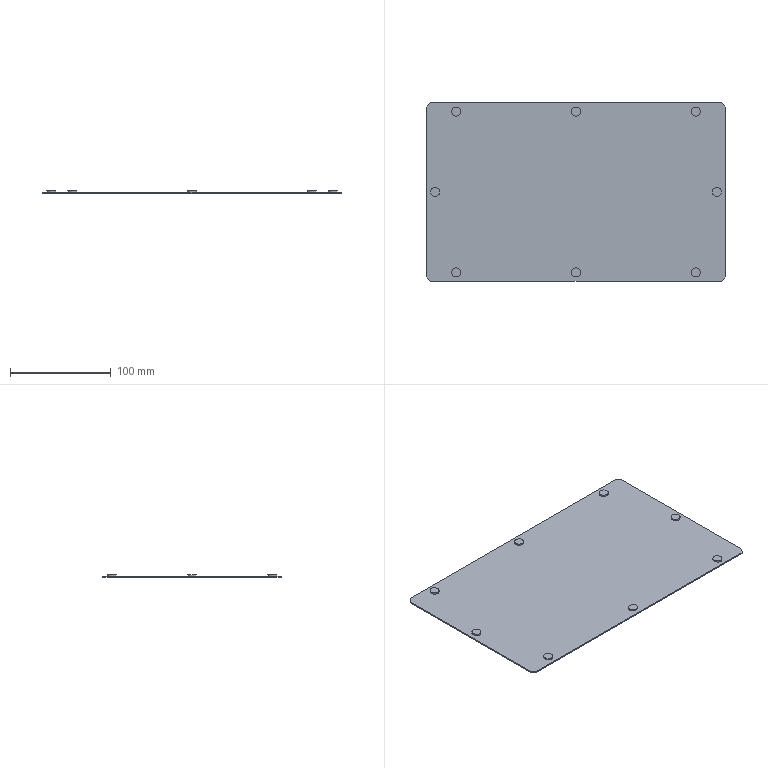Part | SolidWorks | features BaseBody 9 | 9 solids | 58 faces | box 298 x 178 x 2.7 mm | volume 64049 mm3 | cylinder 32 | plane 26 | commonest cylinder face diameters 6.5 x16 9 x16
STEP:
#1=CARTESIAN_POINT('',(123.5,-80.,1.5));
#2=VERTEX_POINT('',#1);
#3=CARTESIAN_POINT('',(114.5,-80.,1.5));
#4=VERTEX_POINT('',#3);
#5=CARTESIAN_POINT('',(119.,-80.,1.5));
#6=DIRECTION('',(0.,0.,1.));
#7=DIRECTION('',(-1.,0.,0.));
#8=AXIS2_PLACEMENT_3D('',#5,#6,#7);
#9=CIRCLE('',#8,4.5);
#10=EDGE_CURVE('',#2,#4,#9,.T.);
#11=ORIENTED_EDGE('',*,*,#10,.F.);
#12=CARTESIAN_POINT('',(123.5,-80.,0.));
#13=VERTEX_POINT('',#12);
#14=CARTESIAN_POINT('',(123.5,-80.,1.5));
#15=DIRECTION('',(0.,0.,-1.));
#16=VECTOR('',#15,1000.);
#17=LINE('',#14,#16);
#18=EDGE_CURVE('',#2,#13,#17,.T.);
#19=ORIENTED_EDGE('',*,*,#18,.T.);
#20=CARTESIAN_POINT('',(114.5,-80.,0.));
#21=VERTEX_POINT('',#20);
#22=CARTESIAN_POINT('',(119.,-80.,0.));
#23=DIRECTION('',(0.,0.,1.));
#24=DIRECTION('',(-1.,0.,0.));
#25=AXIS2_PLACEMENT_3D('',#22,#23,#24);
#26=CIRCLE('',#25,4.5);
#27=EDGE_CURVE('',#13,#21,#26,.T.);
#28=ORIENTED_EDGE('',*,*,#27,.T.);
#29=CARTESIAN_POINT('',(114.5,-80.,1.5));
#30=DIRECTION('',(0.,0.,-1.));
#31=VECTOR('',#30,1000.);
#32=LINE('',#29,#31);
#33=EDGE_CURVE('',#4,#21,#32,.T.);
#34=ORIENTED_EDGE('',*,*,#33,.F.);
#35=EDGE_LOOP('',(#11,#19,#28,#34));
#36=FACE_OUTER_BOUND('',#35,.T.);
#37=CARTESIAN_POINT('',(119.,-80.,1.5));
#38=DIRECTION('',(0.,0.,-1.));
#39=DIRECTION('',(-1.,0.,0.));
#40=AXIS2_PLACEMENT_3D('',#37,#38,#39);
#41=CYLINDRICAL_SURFACE('',#40,4.5);
#42=ADVANCED_FACE('',(#36),#41,.T.);
#43=CARTESIAN_POINT('',(119.,-80.,1.5));
#44=DIRECTION('',(0.,0.,1.));
#45=DIRECTION('',(-1.,0.,0.));
#46=AXIS2_PLACEMENT_3D('',#43,#44,#45);
#47=CIRCLE('',#46,4.5);
#48=EDGE_CURVE('',#4,#2,#47,.T.);
#49=ORIENTED_EDGE('',*,*,#48,.T.);
#50=ORIENTED_EDGE('',*,*,#10,.T.);
#51=EDGE_LOOP('',(#49,#50));
#52=FACE_OUTER_BOUND('',#51,.T.);
#53=CARTESIAN_POINT('',(119.,-80.,1.5));
#54=DIRECTION('',(0.,0.,1.));
#55=DIRECTION('',(1.,0.,0.));
#56=AXIS2_PLACEMENT_3D('',#53,#54,#55);
#57=PLANE('',#56);
#58=ADVANCED_FACE('',(#52),#57,.T.);
#59=ORIENTED_EDGE('',*,*,#18,.F.);
#60=ORIENTED_EDGE('',*,*,#48,.F.);
#61=ORIENTED_EDGE('',*,*,#33,.T.);
#62=CARTESIAN_POINT('',(119.,-80.,0.));
#63=DIRECTION('',(0.,0.,1.));
#64=DIRECTION('',(-1.,0.,0.));
#65=AXIS2_PLACEMENT_3D('',#62,#63,#64);
#66=CIRCLE('',#65,4.5);
#67=EDGE_CURVE('',#21,#13,#66,.T.);
#68=ORIENTED_EDGE('',*,*,#67,.T.);
#69=EDGE_LOOP('',(#59,#60,#61,#68));
#70=FACE_OUTER_BOUND('',#69,.T.);
#71=CARTESIAN_POINT('',(119.,-80.,1.5));
#72=DIRECTION('',(0.,0.,-1.));
#73=DIRECTION('',(-1.,0.,0.));
#74=AXIS2_PLACEMENT_3D('',#71,#72,#73);
#75=CYLINDRICAL_SURFACE('',#74,4.5);
#76=ADVANCED_FACE('',(#70),#75,.T.);
#77=ORIENTED_EDGE('',*,*,#67,.F.);
#78=ORIENTED_EDGE('',*,*,#27,.F.);
#79=EDGE_LOOP('',(#77,#78));
#80=FACE_OUTER_BOUND('',#79,.T.);
#81=CARTESIAN_POINT('',(119.,-80.,0.));
#82=DIRECTION('',(0.,0.,1.));
#83=DIRECTION('',(1.,0.,0.));
#84=AXIS2_PLACEMENT_3D('',#81,#82,#83);
#85=PLANE('',#84);
#86=ADVANCED_FACE('',(#80),#85,.F.);
#87=CLOSED_SHELL('',(#42,#58,#76,#86));
#88=MANIFOLD_SOLID_BREP('',#87);
#89=CARTESIAN_POINT('',(-114.5,80.,1.5));
#90=VERTEX_POINT('',#89);
#91=CARTESIAN_POINT('',(-123.5,80.,1.5));
#92=VERTEX_POINT('',#91);
#93=CARTESIAN_POINT('',(-119.,80.,1.5));
#94=DIRECTION('',(0.,0.,1.));
#95=DIRECTION('',(-1.,0.,0.));
#96=AXIS2_PLACEMENT_3D('',#93,#94,#95);
#97=CIRCLE('',#96,4.5);
#98=EDGE_CURVE('',#90,#92,#97,.T.);
#99=ORIENTED_EDGE('',*,*,#98,.F.);
#100=CARTESIAN_POINT('',(-114.5,80.,0.));
#101=VERTEX_POINT('',#100);
#102=CARTESIAN_POINT('',(-114.5,80.,1.5));
#103=DIRECTION('',(0.,0.,-1.));
#104=VECTOR('',#103,1000.);
#105=LINE('',#102,#104);
#106=EDGE_CURVE('',#90,#101,#105,.T.);
#107=ORIENTED_EDGE('',*,*,#106,.T.);
#108=CARTESIAN_POINT('',(-123.5,80.,0.));
#109=VERTEX_POINT('',#108);
#110=CARTESIAN_POINT('',(-119.,80.,0.));
#111=DIRECTION('',(0.,0.,1.));
#112=DIRECTION('',(-1.,0.,0.));
#113=AXIS2_PLACEMENT_3D('',#110,#111,#112);
#114=CIRCLE('',#113,4.5);
#115=EDGE_CURVE('',#101,#109,#114,.T.);
#116=ORIENTED_EDGE('',*,*,#115,.T.);
#117=CARTESIAN_POINT('',(-123.5,80.,1.5));
#118=DIRECTION('',(0.,0.,-1.));
#119=VECTOR('',#118,1000.);
#120=LINE('',#117,#119);
#121=EDGE_CURVE('',#92,#109,#120,.T.);
#122=ORIENTED_EDGE('',*,*,#121,.F.);
#123=EDGE_LOOP('',(#99,#107,#116,#122));
#124=FACE_OUTER_BOUND('',#123,.T.);
#125=CARTESIAN_POINT('',(-119.,80.,1.5));
#126=DIRECTION('',(0.,0.,-1.));
#127=DIRECTION('',(-1.,0.,0.));
#128=AXIS2_PLACEMENT_3D('',#125,#126,#127);
#129=CYLINDRICAL_SURFACE('',#128,4.5);
#130=ADVANCED_FACE('',(#124),#129,.T.);
#131=CARTESIAN_POINT('',(-119.,80.,1.5));
#132=DIRECTION('',(0.,0.,1.));
#133=DIRECTION('',(-1.,0.,0.));
#134=AXIS2_PLACEMENT_3D('',#131,#132,#133);
#135=CIRCLE('',#134,4.5);
#136=EDGE_CURVE('',#92,#90,#135,.T.);
#137=ORIENTED_EDGE('',*,*,#136,.T.);
#138=ORIENTED_EDGE('',*,*,#98,.T.);
#139=EDGE_LOOP('',(#137,#138));
#140=FACE_OUTER_BOUND('',#139,.T.);
#141=CARTESIAN_POINT('',(-119.,80.,1.5));
#142=DIRECTION('',(0.,0.,1.));
#143=DIRECTION('',(1.,0.,0.));
#144=AXIS2_PLACEMENT_3D('',#141,#142,#143);
#145=PLANE('',#144);
#146=ADVANCED_FACE('',(#140),#145,.T.);
#147=ORIENTED_EDGE('',*,*,#106,.F.);
#148=ORIENTED_EDGE('',*,*,#136,.F.);
#149=ORIENTED_EDGE('',*,*,#121,.T.);
#150=CARTESIAN_POINT('',(-119.,80.,0.));
#151=DIRECTION('',(0.,0.,1.));
#152=DIRECTION('',(-1.,0.,0.));
#153=AXIS2_PLACEMENT_3D('',#150,#151,#152);
#154=CIRCLE('',#153,4.5);
#155=EDGE_CURVE('',#109,#101,#154,.T.);
#156=ORIENTED_EDGE('',*,*,#155,.T.);
#157=EDGE_LOOP('',(#147,#148,#149,#156));
#158=FACE_OUTER_BOUND('',#157,.T.);
#159=CARTESIAN_POINT('',(-119.,80.,1.5));
#160=DIRECTION('',(0.,0.,-1.));
#161=DIRECTION('',(-1.,0.,0.));
#162=AXIS2_PLACEMENT_3D('',#159,#160,#161);
#163=CYLINDRICAL_SURFACE('',#162,4.5);
#164=ADVANCED_FACE('',(#158),#163,.T.);
#165=ORIENTED_EDGE('',*,*,#155,.F.);
#166=ORIENTED_EDGE('',*,*,#115,.F.);
#167=EDGE_LOOP('',(#165,#166));
#168=FACE_OUTER_BOUND('',#167,.T.);
#169=CARTESIAN_POINT('',(-119.,80.,0.));
#170=DIRECTION('',(0.,0.,1.));
#171=DIRECTION('',(1.,0.,0.));
#172=AXIS2_PLACEMENT_3D('',#169,#170,#171);
#173=PLANE('',#172);
#174=ADVANCED_FACE('',(#168),#173,.F.);
#175=CLOSED_SHELL('',(#130,#146,#164,#174));
#176=MANIFOLD_SOLID_BREP('',#175);
#177=CARTESIAN_POINT('',(-114.5,-80.,1.5));
#178=VERTEX_POINT('',#177);
#179=CARTESIAN_POINT('',(-123.5,-80.,1.5));
#180=VERTEX_POINT('',#179);
#181=CARTESIAN_POINT('',(-119.,-80.,1.5));
#182=DIRECTION('',(0.,0.,1.));
#183=DIRECTION('',(-1.,0.,0.));
#184=AXIS2_PLACEMENT_3D('',#181,#182,#183);
#185=CIRCLE('',#184,4.5);
#186=EDGE_CURVE('',#178,#180,#185,.T.);
#187=ORIENTED_EDGE('',*,*,#186,.F.);
#188=CARTESIAN_POINT('',(-114.5,-80.,0.));
#189=VERTEX_POINT('',#188);
#190=CARTESIAN_POINT('',(-114.5,-80.,1.5));
#191=DIRECTION('',(0.,0.,-1.));
#192=VECTOR('',#191,1000.);
#193=LINE('',#190,#192);
#194=EDGE_CURVE('',#178,#189,#193,.T.);
#195=ORIENTED_EDGE('',*,*,#194,.T.);
#196=CARTESIAN_POINT('',(-123.5,-80.,0.));
#197=VERTEX_POINT('',#196);
#198=CARTESIAN_POINT('',(-119.,-80.,0.));
#199=DIRECTION('',(0.,0.,1.));
#200=DIRECTION('',(-1.,0.,0.));
#201=AXIS2_PLACEMENT_3D('',#198,#199,#200);
#202=CIRCLE('',#201,4.5);
#203=EDGE_CURVE('',#189,#197,#202,.T.);
#204=ORIENTED_EDGE('',*,*,#203,.T.);
#205=CARTESIAN_POINT('',(-123.5,-80.,1.5));
#206=DIRECTION('',(0.,0.,-1.));
#207=VECTOR('',#206,1000.);
#208=LINE('',#205,#207);
#209=EDGE_CURVE('',#180,#197,#208,.T.);
#210=ORIENTED_EDGE('',*,*,#209,.F.);
#211=EDGE_LOOP('',(#187,#195,#204,#210));
#212=FACE_OUTER_BOUND('',#211,.T.);
#213=CARTESIAN_POINT('',(-119.,-80.,1.5));
#214=DIRECTION('',(0.,0.,-1.));
#215=DIRECTION('',(-1.,0.,0.));
#216=AXIS2_PLACEMENT_3D('',#213,#214,#215);
#217=CYLINDRICAL_SURFACE('',#216,4.5);
#218=ADVANCED_FACE('',(#212),#217,.T.);
#219=CARTESIAN_POINT('',(-119.,-80.,1.5));
#220=DIRECTION('',(0.,0.,1.));
#221=DIRECTION('',(-1.,0.,0.));
#222=AXIS2_PLACEMENT_3D('',#219,#220,#221);
#223=CIRCLE('',#222,4.5);
#224=EDGE_CURVE('',#180,#178,#223,.T.);
#225=ORIENTED_EDGE('',*,*,#224,.T.);
#226=ORIENTED_EDGE('',*,*,#186,.T.);
#227=EDGE_LOOP('',(#225,#226));
#228=FACE_OUTER_BOUND('',#227,.T.);
#229=CARTESIAN_POINT('',(-119.,-80.,1.5));
#230=DIRECTION('',(0.,0.,1.));
#231=DIRECTION('',(1.,0.,0.));
#232=AXIS2_PLACEMENT_3D('',#229,#230,#231);
#233=PLANE('',#232);
#234=ADVANCED_FACE('',(#228),#233,.T.);
#235=ORIENTED_EDGE('',*,*,#194,.F.);
#236=ORIENTED_EDGE('',*,*,#224,.F.);
#237=ORIENTED_EDGE('',*,*,#209,.T.);
#238=CARTESIAN_POINT('',(-119.,-80.,0.));
#239=DIRECTION('',(0.,0.,1.));
#240=DIRECTION('',(-1.,0.,0.));
#241=AXIS2_PLACEMENT_3D('',#238,#239,#240);
#242=CIRCLE('',#241,4.5);
#243=EDGE_CURVE('',#197,#189,#242,.T.);
#244=ORIENTED_EDGE('',*,*,#243,.T.);
#245=EDGE_LOOP('',(#235,#236,#237,#244));
#246=FACE_OUTER_BOUND('',#245,.T.);
#247=CARTESIAN_POINT('',(-119.,-80.,1.5));
#248=DIRECTION('',(0.,0.,-1.));
#249=DIRECTION('',(-1.,0.,0.));
#250=AXIS2_PLACEMENT_3D('',#247,#248,#249);
#251=CYLINDRICAL_SURFACE('',#250,4.5);
#252=ADVANCED_FACE('',(#246),#251,.T.);
#253=ORIENTED_EDGE('',*,*,#243,.F.);
#254=ORIENTED_EDGE('',*,*,#203,.F.);
#255=EDGE_LOOP('',(#253,#254));
#256=FACE_OUTER_BOUND('',#255,.T.);
#257=CARTESIAN_POINT('',(-119.,-80.,0.));
#258=DIRECTION('',(0.,0.,1.));
#259=DIRECTION('',(1.,0.,0.));
#260=AXIS2_PLACEMENT_3D('',#257,#258,#259);
#261=PLANE('',#260);
#262=ADVANCED_FACE('',(#256),#261,.F.);
#263=CLOSED_SHELL('',(#218,#234,#252,#262));
#264=MANIFOLD_SOLID_BREP('',#263);
#265=CARTESIAN_POINT('',(-122.25,80.,-1.2));
#266=VERTEX_POINT('',#265);
#267=CARTESIAN_POINT('',(-115.75,80.,-1.2));
#268=VERTEX_POINT('',#267);
#269=CARTESIAN_POINT('',(-119.,80.,-1.2));
#270=DIRECTION('',(0.,0.,1.));
#271=DIRECTION('',(1.,0.,0.));
#272=AXIS2_PLACEMENT_3D('',#269,#270,#271);
#273=CIRCLE('',#272,3.25);
#274=EDGE_CURVE('',#266,#268,#273,.T.);
#275=ORIENTED_EDGE('',*,*,#274,.F.);
#276=CARTESIAN_POINT('',(-122.25,80.,0.));
#277=VERTEX_POINT('',#276);
#278=CARTESIAN_POINT('',(-122.25,80.,-1.2));
#279=DIRECTION('',(0.,0.,1.));
#280=VECTOR('',#279,1000.);
#281=LINE('',#278,#280);
#282=EDGE_CURVE('',#266,#277,#281,.T.);
#283=ORIENTED_EDGE('',*,*,#282,.T.);
#284=CARTESIAN_POINT('',(-115.75,80.,0.));
#285=VERTEX_POINT('',#284);
#286=CARTESIAN_POINT('',(-119.,80.,0.));
#287=DIRECTION('',(0.,0.,-1.));
#288=DIRECTION('',(1.,0.,0.));
#289=AXIS2_PLACEMENT_3D('',#286,#287,#288);
#290=CIRCLE('',#289,3.25);
#291=EDGE_CURVE('',#285,#277,#290,.T.);
#292=ORIENTED_EDGE('',*,*,#291,.F.);
#293=CARTESIAN_POINT('',(-115.75,80.,-1.2));
#294=DIRECTION('',(0.,0.,1.));
#295=VECTOR('',#294,1000.);
#296=LINE('',#293,#295);
#297=EDGE_CURVE('',#268,#285,#296,.T.);
#298=ORIENTED_EDGE('',*,*,#297,.F.);
#299=EDGE_LOOP('',(#275,#283,#292,#298));
#300=FACE_OUTER_BOUND('',#299,.T.);
#301=CARTESIAN_POINT('',(-119.,80.,-1.2));
#302=DIRECTION('',(0.,0.,1.));
#303=DIRECTION('',(1.,0.,0.));
#304=AXIS2_PLACEMENT_3D('',#301,#302,#303);
#305=CYLINDRICAL_SURFACE('',#304,3.25);
#306=ADVANCED_FACE('',(#300),#305,.F.);
#307=CARTESIAN_POINT('',(-143.25,0.,-1.2));
#308=VERTEX_POINT('',#307);
#309=CARTESIAN_POINT('',(-136.75,0.,-1.2));
#310=VERTEX_POINT('',#309);
#311=CARTESIAN_POINT('',(-140.,0.,-1.2));
#312=DIRECTION('',(0.,0.,1.));
#313=DIRECTION('',(1.,0.,0.));
#314=AXIS2_PLACEMENT_3D('',#311,#312,#313);
#315=CIRCLE('',#314,3.25);
#316=EDGE_CURVE('',#308,#310,#315,.T.);
#317=ORIENTED_EDGE('',*,*,#316,.F.);
#318=CARTESIAN_POINT('',(-143.25,0.,0.));
#319=VERTEX_POINT('',#318);
#320=CARTESIAN_POINT('',(-143.25,0.,-1.2));
#321=DIRECTION('',(0.,0.,1.));
#322=VECTOR('',#321,1000.);
#323=LINE('',#320,#322);
#324=EDGE_CURVE('',#308,#319,#323,.T.);
#325=ORIENTED_EDGE('',*,*,#324,.T.);
#326=CARTESIAN_POINT('',(-136.75,0.,0.));
#327=VERTEX_POINT('',#326);
#328=CARTESIAN_POINT('',(-140.,0.,0.));
#329=DIRECTION('',(0.,0.,-1.));
#330=DIRECTION('',(1.,0.,0.));
#331=AXIS2_PLACEMENT_3D('',#328,#329,#330);
#332=CIRCLE('',#331,3.25);
#333=EDGE_CURVE('',#327,#319,#332,.T.);
#334=ORIENTED_EDGE('',*,*,#333,.F.);
#335=CARTESIAN_POINT('',(-136.75,0.,-1.2));
#336=DIRECTION('',(0.,0.,1.));
#337=VECTOR('',#336,1000.);
#338=LINE('',#335,#337);
#339=EDGE_CURVE('',#310,#327,#338,.T.);
#340=ORIENTED_EDGE('',*,*,#339,.F.);
#341=EDGE_LOOP('',(#317,#325,#334,#340));
#342=FACE_OUTER_BOUND('',#341,.T.);
#343=CARTESIAN_POINT('',(-140.,0.,-1.2));
#344=DIRECTION('',(0.,0.,1.));
#345=DIRECTION('',(1.,0.,0.));
#346=AXIS2_PLACEMENT_3D('',#343,#344,#345);
#347=CYLINDRICAL_SURFACE('',#346,3.25);
#348=ADVANCED_FACE('',(#342),#347,.F.);
#349=CARTESIAN_POINT('',(-122.25,-80.,-1.2));
#350=VERTEX_POINT('',#349);
#351=CARTESIAN_POINT('',(-115.75,-80.,-1.2));
#352=VERTEX_POINT('',#351);
#353=CARTESIAN_POINT('',(-119.,-80.,-1.2));
#354=DIRECTION('',(0.,0.,1.));
#355=DIRECTION('',(1.,0.,0.));
#356=AXIS2_PLACEMENT_3D('',#353,#354,#355);
#357=CIRCLE('',#356,3.25);
#358=EDGE_CURVE('',#350,#352,#357,.T.);
#359=ORIENTED_EDGE('',*,*,#358,.F.);
#360=CARTESIAN_POINT('',(-122.25,-80.,0.));
#361=VERTEX_POINT('',#360);
#362=CARTESIAN_POINT('',(-122.25,-80.,-1.2));
#363=DIRECTION('',(0.,0.,1.));
#364=VECTOR('',#363,1000.);
#365=LINE('',#362,#364);
#366=EDGE_CURVE('',#350,#361,#365,.T.);
#367=ORIENTED_EDGE('',*,*,#366,.T.);
#368=CARTESIAN_POINT('',(-115.75,-80.,0.));
#369=VERTEX_POINT('',#368);
#370=CARTESIAN_POINT('',(-119.,-80.,0.));
#371=DIRECTION('',(0.,0.,-1.));
#372=DIRECTION('',(1.,0.,0.));
#373=AXIS2_PLACEMENT_3D('',#370,#371,#372);
#374=CIRCLE('',#373,3.25);
#375=EDGE_CURVE('',#369,#361,#374,.T.);
#376=ORIENTED_EDGE('',*,*,#375,.F.);
#377=CARTESIAN_POINT('',(-115.75,-80.,-1.2));
#378=DIRECTION('',(0.,0.,1.));
#379=VECTOR('',#378,1000.);
#380=LINE('',#377,#379);
#381=EDGE_CURVE('',#352,#369,#380,.T.);
#382=ORIENTED_EDGE('',*,*,#381,.F.);
#383=EDGE_LOOP('',(#359,#367,#376,#382));
#384=FACE_OUTER_BOUND('',#383,.T.);
#385=CARTESIAN_POINT('',(-119.,-80.,-1.2));
#386=DIRECTION('',(0.,0.,1.));
#387=DIRECTION('',(1.,0.,0.));
#388=AXIS2_PLACEMENT_3D('',#385,#386,#387);
#389=CYLINDRICAL_SURFACE('',#388,3.25);
#390=ADVANCED_FACE('',(#384),#389,.F.);
#391=CARTESIAN_POINT('',(-3.25,80.,-1.2));
#392=VERTEX_POINT('',#391);
#393=CARTESIAN_POINT('',(3.25,80.,-1.2));
#394=VERTEX_POINT('',#393);
#395=CARTESIAN_POINT('',(0.,80.,-1.2));
#396=DIRECTION('',(0.,0.,1.));
#397=DIRECTION('',(1.,0.,0.));
#398=AXIS2_PLACEMENT_3D('',#395,#396,#397);
#399=CIRCLE('',#398,3.25);
#400=EDGE_CURVE('',#392,#394,#399,.T.);
#401=ORIENTED_EDGE('',*,*,#400,.F.);
#402=CARTESIAN_POINT('',(-3.25,80.,0.));
#403=VERTEX_POINT('',#402);
#404=CARTESIAN_POINT('',(-3.25,80.,-1.2));
#405=DIRECTION('',(0.,0.,1.));
#406=VECTOR('',#405,1000.);
#407=LINE('',#404,#406);
#408=EDGE_CURVE('',#392,#403,#407,.T.);
#409=ORIENTED_EDGE('',*,*,#408,.T.);
#410=CARTESIAN_POINT('',(3.25,80.,0.));
#411=VERTEX_POINT('',#410);
#412=CARTESIAN_POINT('',(0.,80.,0.));
#413=DIRECTION('',(0.,0.,-1.));
#414=DIRECTION('',(1.,0.,0.));
#415=AXIS2_PLACEMENT_3D('',#412,#413,#414);
#416=CIRCLE('',#415,3.25);
#417=EDGE_CURVE('',#411,#403,#416,.T.);
#418=ORIENTED_EDGE('',*,*,#417,.F.);
#419=CARTESIAN_POINT('',(3.25,80.,-1.2));
#420=DIRECTION('',(0.,0.,1.));
#421=VECTOR('',#420,1000.);
#422=LINE('',#419,#421);
#423=EDGE_CURVE('',#394,#411,#422,.T.);
#424=ORIENTED_EDGE('',*,*,#423,.F.);
#425=EDGE_LOOP('',(#401,#409,#418,#424));
#426=FACE_OUTER_BOUND('',#425,.T.);
#427=CARTESIAN_POINT('',(0.,80.,-1.2));
#428=DIRECTION('',(0.,0.,1.));
#429=DIRECTION('',(1.,0.,0.));
#430=AXIS2_PLACEMENT_3D('',#427,#428,#429);
#431=CYLINDRICAL_SURFACE('',#430,3.25);
#432=ADVANCED_FACE('',(#426),#431,.F.);
#433=CARTESIAN_POINT('',(-3.25,-80.,-1.2));
#434=VERTEX_POINT('',#433);
#435=CARTESIAN_POINT('',(3.25,-80.,-1.2));
#436=VERTEX_POINT('',#435);
#437=CARTESIAN_POINT('',(0.,-80.,-1.2));
#438=DIRECTION('',(0.,0.,1.));
#439=DIRECTION('',(1.,0.,0.));
#440=AXIS2_PLACEMENT_3D('',#437,#438,#439);
#441=CIRCLE('',#440,3.25);
#442=EDGE_CURVE('',#434,#436,#441,.T.);
#443=ORIENTED_EDGE('',*,*,#442,.F.);
#444=CARTESIAN_POINT('',(-3.25,-80.,0.));
#445=VERTEX_POINT('',#444);
#446=CARTESIAN_POINT('',(-3.25,-80.,-1.2));
#447=DIRECTION('',(0.,0.,1.));
#448=VECTOR('',#447,1000.);
#449=LINE('',#446,#448);
#450=EDGE_CURVE('',#434,#445,#449,.T.);
#451=ORIENTED_EDGE('',*,*,#450,.T.);
#452=CARTESIAN_POINT('',(3.25,-80.,0.));
#453=VERTEX_POINT('',#452);
#454=CARTESIAN_POINT('',(0.,-80.,0.));
#455=DIRECTION('',(0.,0.,-1.));
#456=DIRECTION('',(1.,0.,0.));
#457=AXIS2_PLACEMENT_3D('',#454,#455,#456);
#458=CIRCLE('',#457,3.25);
#459=EDGE_CURVE('',#453,#445,#458,.T.);
#460=ORIENTED_EDGE('',*,*,#459,.F.);
#461=CARTESIAN_POINT('',(3.25,-80.,-1.2));
#462=DIRECTION('',(0.,0.,1.));
#463=VECTOR('',#462,1000.);
#464=LINE('',#461,#463);
#465=EDGE_CURVE('',#436,#453,#464,.T.);
#466=ORIENTED_EDGE('',*,*,#465,.F.);
#467=EDGE_LOOP('',(#443,#451,#460,#466));
#468=FACE_OUTER_BOUND('',#467,.T.);
#469=CARTESIAN_POINT('',(0.,-80.,-1.2));
#470=DIRECTION('',(0.,0.,1.));
#471=DIRECTION('',(1.,0.,0.));
#472=AXIS2_PLACEMENT_3D('',#469,#470,#471);
#473=CYLINDRICAL_SURFACE('',#472,3.25);
#474=ADVANCED_FACE('',(#468),#473,.F.);
#475=CARTESIAN_POINT('',(115.75,-80.,-1.2));
#476=VERTEX_POINT('',#475);
#477=CARTESIAN_POINT('',(122.25,-80.,-1.2));
#478=VERTEX_POINT('',#477);
#479=CARTESIAN_POINT('',(119.,-80.,-1.2));
#480=DIRECTION('',(0.,0.,1.));
#481=DIRECTION('',(1.,0.,0.));
#482=AXIS2_PLACEMENT_3D('',#479,#480,#481);
#483=CIRCLE('',#482,3.25);
#484=EDGE_CURVE('',#476,#478,#483,.T.);
#485=ORIENTED_EDGE('',*,*,#484,.F.);
#486=CARTESIAN_POINT('',(115.75,-80.,0.));
#487=VERTEX_POINT('',#486);
#488=CARTESIAN_POINT('',(115.75,-80.,-1.2));
#489=DIRECTION('',(0.,0.,1.));
#490=VECTOR('',#489,1000.);
#491=LINE('',#488,#490);
#492=EDGE_CURVE('',#476,#487,#491,.T.);
#493=ORIENTED_EDGE('',*,*,#492,.T.);
#494=CARTESIAN_POINT('',(122.25,-80.,0.));
#495=VERTEX_POINT('',#494);
#496=CARTESIAN_POINT('',(119.,-80.,0.));
#497=DIRECTION('',(0.,0.,-1.));
#498=DIRECTION('',(1.,0.,0.));
#499=AXIS2_PLACEMENT_3D('',#496,#497,#498);
#500=CIRCLE('',#499,3.25);
#501=EDGE_CURVE('',#495,#487,#500,.T.);
#502=ORIENTED_EDGE('',*,*,#501,.F.);
#503=CARTESIAN_POINT('',(122.25,-80.,-1.2));
#504=DIRECTION('',(0.,0.,1.));
#505=VECTOR('',#504,1000.);
#506=LINE('',#503,#505);
#507=EDGE_CURVE('',#478,#495,#506,.T.);
#508=ORIENTED_EDGE('',*,*,#507,.F.);
#509=EDGE_LOOP('',(#485,#493,#502,#508));
#510=FACE_OUTER_BOUND('',#509,.T.);
#511=CARTESIAN_POINT('',(119.,-80.,-1.2));
#512=DIRECTION('',(0.,0.,1.));
#513=DIRECTION('',(1.,0.,0.));
#514=AXIS2_PLACEMENT_3D('',#511,#512,#513);
#515=CYLINDRICAL_SURFACE('',#514,3.25);
#516=ADVANCED_FACE('',(#510),#515,.F.);
#517=CARTESIAN_POINT('',(115.75,80.,-1.2));
#518=VERTEX_POINT('',#517);
#519=CARTESIAN_POINT('',(122.25,80.,-1.2));
#520=VERTEX_POINT('',#519);
#521=CARTESIAN_POINT('',(119.,80.,-1.2));
#522=DIRECTION('',(0.,0.,1.));
#523=DIRECTION('',(1.,0.,0.));
#524=AXIS2_PLACEMENT_3D('',#521,#522,#523);
#525=CIRCLE('',#524,3.25);
#526=EDGE_CURVE('',#518,#520,#525,.T.);
#527=ORIENTED_EDGE('',*,*,#526,.F.);
#528=CARTESIAN_POINT('',(115.75,80.,0.));
#529=VERTEX_POINT('',#528);
#530=CARTESIAN_POINT('',(115.75,80.,-1.2));
#531=DIRECTION('',(0.,0.,1.));
#532=VECTOR('',#531,1000.);
#533=LINE('',#530,#532);
#534=EDGE_CURVE('',#518,#529,#533,.T.);
#535=ORIENTED_EDGE('',*,*,#534,.T.);
#536=CARTESIAN_POINT('',(122.25,80.,0.));
#537=VERTEX_POINT('',#536);
#538=CARTESIAN_POINT('',(119.,80.,0.));
#539=DIRECTION('',(0.,0.,-1.));
#540=DIRECTION('',(1.,0.,0.));
#541=AXIS2_PLACEMENT_3D('',#538,#539,#540);
#542=CIRCLE('',#541,3.25);
#543=EDGE_CURVE('',#537,#529,#542,.T.);
#544=ORIENTED_EDGE('',*,*,#543,.F.);
#545=CARTESIAN_POINT('',(122.25,80.,-1.2));
#546=DIRECTION('',(0.,0.,1.));
#547=VECTOR('',#546,1000.);
#548=LINE('',#545,#547);
#549=EDGE_CURVE('',#520,#537,#548,.T.);
#550=ORIENTED_EDGE('',*,*,#549,.F.);
#551=EDGE_LOOP('',(#527,#535,#544,#550));
#552=FACE_OUTER_BOUND('',#551,.T.);
#553=CARTESIAN_POINT('',(119.,80.,-1.2));
#554=DIRECTION('',(0.,0.,1.));
#555=DIRECTION('',(1.,0.,0.));
#556=AXIS2_PLACEMENT_3D('',#553,#554,#555);
#557=CYLINDRICAL_SURFACE('',#556,3.25);
#558=ADVANCED_FACE('',(#552),#557,.F.);
#559=CARTESIAN_POINT('',(136.75,0.,-1.2));
#560=VERTEX_POINT('',#559);
#561=CARTESIAN_POINT('',(143.25,0.,-1.2));
#562=VERTEX_POINT('',#561);
#563=CARTESIAN_POINT('',(140.,0.,-1.2));
#564=DIRECTION('',(0.,0.,1.));
#565=DIRECTION('',(1.,0.,0.));
#566=AXIS2_PLACEMENT_3D('',#563,#564,#565);
#567=CIRCLE('',#566,3.25);
#568=EDGE_CURVE('',#560,#562,#567,.T.);
#569=ORIENTED_EDGE('',*,*,#568,.F.);
#570=CARTESIAN_POINT('',(136.75,0.,0.));
#571=VERTEX_POINT('',#570);
#572=CARTESIAN_POINT('',(136.75,0.,-1.2));
#573=DIRECTION('',(0.,0.,1.));
#574=VECTOR('',#573,1000.);
#575=LINE('',#572,#574);
#576=EDGE_CURVE('',#560,#571,#575,.T.);
#577=ORIENTED_EDGE('',*,*,#576,.T.);
#578=CARTESIAN_POINT('',(143.25,0.,0.));
#579=VERTEX_POINT('',#578);
#580=CARTESIAN_POINT('',(140.,0.,0.));
#581=DIRECTION('',(0.,0.,-1.));
#582=DIRECTION('',(1.,0.,0.));
#583=AXIS2_PLACEMENT_3D('',#580,#581,#582);
#584=CIRCLE('',#583,3.25);
#585=EDGE_CURVE('',#579,#571,#584,.T.);
#586=ORIENTED_EDGE('',*,*,#585,.F.);
#587=CARTESIAN_POINT('',(143.25,0.,-1.2));
#588=DIRECTION('',(0.,0.,1.));
#589=VECTOR('',#588,1000.);
#590=LINE('',#587,#589);
#591=EDGE_CURVE('',#562,#579,#590,.T.);
#592=ORIENTED_EDGE('',*,*,#591,.F.);
#593=EDGE_LOOP('',(#569,#577,#586,#592));
#594=FACE_OUTER_BOUND('',#593,.T.);
#595=CARTESIAN_POINT('',(140.,0.,-1.2));
#596=DIRECTION('',(0.,0.,1.));
#597=DIRECTION('',(1.,0.,0.));
#598=AXIS2_PLACEMENT_3D('',#595,#596,#597);
#599=CYLINDRICAL_SURFACE('',#598,3.25);
#600=ADVANCED_FACE('',(#594),#599,.F.);
#601=CARTESIAN_POINT('',(-144.5,-89.,0.));
#602=VERTEX_POINT('',#601);
#603=CARTESIAN_POINT('',(144.5,-89.,0.));
#604=VERTEX_POINT('',#603);
#605=CARTESIAN_POINT('',(0.,-89.,0.));
#606=DIRECTION('',(1.,0.,0.));
#607=VECTOR('',#606,1000.);
#608=LINE('',#605,#607);
#609=EDGE_CURVE('',#602,#604,#608,.T.);
#610=ORIENTED_EDGE('',*,*,#609,.T.);
#611=CARTESIAN_POINT('',(149.,-84.5,0.));
#612=VERTEX_POINT('',#611);
#613=CARTESIAN_POINT('',(144.5,-89.,0.));
#614=DIRECTION('',(0.7071,0.7071,0.));
#615=VECTOR('',#614,1000.);
#616=LINE('',#613,#615);
#617=EDGE_CURVE('',#604,#612,#616,.T.);
#618=ORIENTED_EDGE('',*,*,#617,.T.);
#619=CARTESIAN_POINT('',(149.,84.5,0.));
#620=VERTEX_POINT('',#619);
#621=CARTESIAN_POINT('',(149.,0.,0.));
#622=DIRECTION('',(0.,1.,0.));
#623=VECTOR('',#622,1000.);
#624=LINE('',#621,#623);
#625=EDGE_CURVE('',#612,#620,#624,.T.);
#626=ORIENTED_EDGE('',*,*,#625,.T.);
#627=CARTESIAN_POINT('',(144.5,89.,0.));
#628=VERTEX_POINT('',#627);
#629=CARTESIAN_POINT('',(149.,84.5,0.));
#630=DIRECTION('',(-0.7071,0.7071,0.));
#631=VECTOR('',#630,1000.);
#632=LINE('',#629,#631);
#633=EDGE_CURVE('',#620,#628,#632,.T.);
#634=ORIENTED_EDGE('',*,*,#633,.T.);
#635=CARTESIAN_POINT('',(-144.5,89.,0.));
#636=VERTEX_POINT('',#635);
#637=CARTESIAN_POINT('',(0.,89.,0.));
#638=DIRECTION('',(-1.,0.,0.));
#639=VECTOR('',#638,1000.);
#640=LINE('',#637,#639);
#641=EDGE_CURVE('',#628,#636,#640,.T.);
#642=ORIENTED_EDGE('',*,*,#641,.T.);
#643=CARTESIAN_POINT('',(-149.,84.5,0.));
#644=VERTEX_POINT('',#643);
#645=CARTESIAN_POINT('',(-144.5,89.,0.));
#646=DIRECTION('',(-0.7071,-0.7071,0.));
#647=VECTOR('',#646,1000.);
#648=LINE('',#645,#647);
#649=EDGE_CURVE('',#636,#644,#648,.T.);
#650=ORIENTED_EDGE('',*,*,#649,.T.);
#651=CARTESIAN_POINT('',(-149.,-84.5,0.));
#652=VERTEX_POINT('',#651);
#653=CARTESIAN_POINT('',(-149.,0.,0.));
#654=DIRECTION('',(0.,-1.,0.));
#655=VECTOR('',#654,1000.);
#656=LINE('',#653,#655);
#657=EDGE_CURVE('',#644,#652,#656,.T.);
#658=ORIENTED_EDGE('',*,*,#657,.T.);
#659=CARTESIAN_POINT('',(-149.,-84.5,0.));
#660=DIRECTION('',(0.7071,-0.7071,0.));
#661=VECTOR('',#660,1000.);
#662=LINE('',#659,#661);
#663=EDGE_CURVE('',#652,#602,#662,.T.);
#664=ORIENTED_EDGE('',*,*,#663,.T.);
#665=EDGE_LOOP('',(#610,#618,#626,#634,#642,#650,#658,#664));
#666=FACE_OUTER_BOUND('',#665,.T.);
#667=ORIENTED_EDGE('',*,*,#291,.T.);
#668=CARTESIAN_POINT('',(-119.,80.,0.));
#669=DIRECTION('',(0.,0.,-1.));
#670=DIRECTION('',(1.,0.,0.));
#671=AXIS2_PLACEMENT_3D('',#668,#669,#670);
#672=CIRCLE('',#671,3.25);
#673=EDGE_CURVE('',#277,#285,#672,.T.);
#674=ORIENTED_EDGE('',*,*,#673,.T.);
#675=EDGE_LOOP('',(#667,#674));
#676=FACE_BOUND('',#675,.T.);
#677=ORIENTED_EDGE('',*,*,#333,.T.);
#678=CARTESIAN_POINT('',(-140.,0.,0.));
#679=DIRECTION('',(0.,0.,-1.));
#680=DIRECTION('',(1.,0.,0.));
#681=AXIS2_PLACEMENT_3D('',#678,#679,#680);
#682=CIRCLE('',#681,3.25);
#683=EDGE_CURVE('',#319,#327,#682,.T.);
#684=ORIENTED_EDGE('',*,*,#683,.T.);
#685=EDGE_LOOP('',(#677,#684));
#686=FACE_BOUND('',#685,.T.);
#687=ORIENTED_EDGE('',*,*,#375,.T.);
#688=CARTESIAN_POINT('',(-119.,-80.,0.));
#689=DIRECTION('',(0.,0.,-1.));
#690=DIRECTION('',(1.,0.,0.));
#691=AXIS2_PLACEMENT_3D('',#688,#689,#690);
#692=CIRCLE('',#691,3.25);
#693=EDGE_CURVE('',#361,#369,#692,.T.);
#694=ORIENTED_EDGE('',*,*,#693,.T.);
#695=EDGE_LOOP('',(#687,#694));
#696=FACE_BOUND('',#695,.T.);
#697=ORIENTED_EDGE('',*,*,#417,.T.);
#698=CARTESIAN_POINT('',(0.,80.,0.));
#699=DIRECTION('',(0.,0.,-1.));
#700=DIRECTION('',(1.,0.,0.));
#701=AXIS2_PLACEMENT_3D('',#698,#699,#700);
#702=CIRCLE('',#701,3.25);
#703=EDGE_CURVE('',#403,#411,#702,.T.);
#704=ORIENTED_EDGE('',*,*,#703,.T.);
#705=EDGE_LOOP('',(#697,#704));
#706=FACE_BOUND('',#705,.T.);
#707=ORIENTED_EDGE('',*,*,#459,.T.);
#708=CARTESIAN_POINT('',(0.,-80.,0.));
#709=DIRECTION('',(0.,0.,-1.));
#710=DIRECTION('',(1.,0.,0.));
#711=AXIS2_PLACEMENT_3D('',#708,#709,#710);
#712=CIRCLE('',#711,3.25);
#713=EDGE_CURVE('',#445,#453,#712,.T.);
#714=ORIENTED_EDGE('',*,*,#713,.T.);
#715=EDGE_LOOP('',(#707,#714));
#716=FACE_BOUND('',#715,.T.);
#717=ORIENTED_EDGE('',*,*,#501,.T.);
#718=CARTESIAN_POINT('',(119.,-80.,0.));
#719=DIRECTION('',(0.,0.,-1.));
#720=DIRECTION('',(1.,0.,0.));
#721=AXIS2_PLACEMENT_3D('',#718,#719,#720);
#722=CIRCLE('',#721,3.25);
#723=EDGE_CURVE('',#487,#495,#722,.T.);
#724=ORIENTED_EDGE('',*,*,#723,.T.);
#725=EDGE_LOOP('',(#717,#724));
#726=FACE_BOUND('',#725,.T.);
#727=ORIENTED_EDGE('',*,*,#543,.T.);
#728=CARTESIAN_POINT('',(119.,80.,0.));
#729=DIRECTION('',(0.,0.,-1.));
#730=DIRECTION('',(1.,0.,0.));
#731=AXIS2_PLACEMENT_3D('',#728,#729,#730);
#732=CIRCLE('',#731,3.25);
#733=EDGE_CURVE('',#529,#537,#732,.T.);
#734=ORIENTED_EDGE('',*,*,#733,.T.);
#735=EDGE_LOOP('',(#727,#734));
#736=FACE_BOUND('',#735,.T.);
#737=ORIENTED_EDGE('',*,*,#585,.T.);
#738=CARTESIAN_POINT('',(140.,0.,0.));
#739=DIRECTION('',(0.,0.,-1.));
#740=DIRECTION('',(1.,0.,0.));
#741=AXIS2_PLACEMENT_3D('',#738,#739,#740);
#742=CIRCLE('',#741,3.25);
#743=EDGE_CURVE('',#571,#579,#742,.T.);
#744=ORIENTED_EDGE('',*,*,#743,.T.);
#745=EDGE_LOOP('',(#737,#744));
#746=FACE_BOUND('',#745,.T.);
#747=CARTESIAN_POINT('',(0.,0.,0.));
#748=DIRECTION('',(0.,0.,1.));
#749=DIRECTION('',(1.,0.,0.));
#750=AXIS2_PLACEMENT_3D('',#747,#748,#749);
#751=PLANE('',#750);
#752=ADVANCED_FACE('',(#666,#676,#686,#696,#706,#716,#726,#736,#746),#751,.T.);
#753=CARTESIAN_POINT('',(149.,-84.5,-1.2));
#754=VERTEX_POINT('',#753);
#755=CARTESIAN_POINT('',(149.,-84.5,-1.2));
#756=DIRECTION('',(0.,0.,-1.));
#757=VECTOR('',#756,1000.);
#758=LINE('',#755,#757);
#759=EDGE_CURVE('',#612,#754,#758,.T.);
#760=ORIENTED_EDGE('',*,*,#759,.F.);
#761=ORIENTED_EDGE('',*,*,#617,.F.);
#762=CARTESIAN_POINT('',(144.5,-89.,-1.2));
#763=VERTEX_POINT('',#762);
#764=CARTESIAN_POINT('',(144.5,-89.,-1.2));
#765=DIRECTION('',(0.,0.,1.));
#766=VECTOR('',#765,1000.);
#767=LINE('',#764,#766);
#768=EDGE_CURVE('',#763,#604,#767,.T.);
#769=ORIENTED_EDGE('',*,*,#768,.F.);
#770=CARTESIAN_POINT('',(144.5,-89.,-1.2));
#771=DIRECTION('',(-0.7071,-0.7071,0.));
#772=VECTOR('',#771,1000.);
#773=LINE('',#770,#772);
#774=EDGE_CURVE('',#754,#763,#773,.T.);
#775=ORIENTED_EDGE('',*,*,#774,.F.);
#776=EDGE_LOOP('',(#760,#761,#769,#775));
#777=FACE_OUTER_BOUND('',#776,.T.);
#778=CARTESIAN_POINT('',(144.5,-89.,-1.2));
#779=DIRECTION('',(-0.7071,0.7071,0.));
#780=DIRECTION('',(-0.7071,-0.7071,0.));
#781=AXIS2_PLACEMENT_3D('',#778,#779,#780);
#782=PLANE('',#781);
#783=ADVANCED_FACE('',(#777),#782,.F.);
#784=ORIENTED_EDGE('',*,*,#609,.F.);
#785=CARTESIAN_POINT('',(-144.5,-89.,-1.2));
#786=VERTEX_POINT('',#785);
#787=CARTESIAN_POINT('',(-144.5,-89.,-1.2));
#788=DIRECTION('',(0.,0.,-1.));
#789=VECTOR('',#788,1000.);
#790=LINE('',#787,#789);
#791=EDGE_CURVE('',#602,#786,#790,.T.);
#792=ORIENTED_EDGE('',*,*,#791,.T.);
#793=CARTESIAN_POINT('',(-149.,-89.,-1.2));
#794=DIRECTION('',(1.,0.,0.));
#795=VECTOR('',#794,1000.);
#796=LINE('',#793,#795);
#797=EDGE_CURVE('',#786,#763,#796,.T.);
#798=ORIENTED_EDGE('',*,*,#797,.T.);
#799=ORIENTED_EDGE('',*,*,#768,.T.);
#800=EDGE_LOOP('',(#784,#792,#798,#799));
#801=FACE_OUTER_BOUND('',#800,.T.);
#802=CARTESIAN_POINT('',(-149.,-89.,-1.2));
#803=DIRECTION('',(0.,-1.,0.));
#804=DIRECTION('',(0.,0.,-1.));
#805=AXIS2_PLACEMENT_3D('',#802,#803,#804);
#806=PLANE('',#805);
#807=ADVANCED_FACE('',(#801),#806,.T.);
#808=ORIENTED_EDGE('',*,*,#791,.F.);
#809=ORIENTED_EDGE('',*,*,#663,.F.);
#810=CARTESIAN_POINT('',(-149.,-84.5,-1.2));
#811=VERTEX_POINT('',#810);
#812=CARTESIAN_POINT('',(-149.,-84.5,-1.2));
#813=DIRECTION('',(0.,0.,1.));
#814=VECTOR('',#813,1000.);
#815=LINE('',#812,#814);
#816=EDGE_CURVE('',#811,#652,#815,.T.);
#817=ORIENTED_EDGE('',*,*,#816,.F.);
#818=CARTESIAN_POINT('',(-149.,-84.5,-1.2));
#819=DIRECTION('',(-0.7071,0.7071,0.));
#820=VECTOR('',#819,1000.);
#821=LINE('',#818,#820);
#822=EDGE_CURVE('',#786,#811,#821,.T.);
#823=ORIENTED_EDGE('',*,*,#822,.F.);
#824=EDGE_LOOP('',(#808,#809,#817,#823));
#825=FACE_OUTER_BOUND('',#824,.T.);
#826=CARTESIAN_POINT('',(-149.,-84.5,-1.2));
#827=DIRECTION('',(0.7071,0.7071,0.));
#828=DIRECTION('',(-0.7071,0.7071,0.));
#829=AXIS2_PLACEMENT_3D('',#826,#827,#828);
#830=PLANE('',#829);
#831=ADVANCED_FACE('',(#825),#830,.F.);
#832=ORIENTED_EDGE('',*,*,#657,.F.);
#833=CARTESIAN_POINT('',(-149.,84.5,-1.2));
#834=VERTEX_POINT('',#833);
#835=CARTESIAN_POINT('',(-149.,84.5,-1.2));
#836=DIRECTION('',(0.,0.,-1.));
#837=VECTOR('',#836,1000.);
#838=LINE('',#835,#837);
#839=EDGE_CURVE('',#644,#834,#838,.T.);
#840=ORIENTED_EDGE('',*,*,#839,.T.);
#841=CARTESIAN_POINT('',(-149.,89.,-1.2));
#842=DIRECTION('',(0.,-1.,0.));
#843=VECTOR('',#842,1000.);
#844=LINE('',#841,#843);
#845=EDGE_CURVE('',#834,#811,#844,.T.);
#846=ORIENTED_EDGE('',*,*,#845,.T.);
#847=ORIENTED_EDGE('',*,*,#816,.T.);
#848=EDGE_LOOP('',(#832,#840,#846,#847));
#849=FACE_OUTER_BOUND('',#848,.T.);
#850=CARTESIAN_POINT('',(-149.,89.,-1.2));
#851=DIRECTION('',(-1.,0.,0.));
#852=DIRECTION('',(0.,-1.,0.));
#853=AXIS2_PLACEMENT_3D('',#850,#851,#852);
#854=PLANE('',#853);
#855=ADVANCED_FACE('',(#849),#854,.T.);
#856=ORIENTED_EDGE('',*,*,#839,.F.);
#857=ORIENTED_EDGE('',*,*,#649,.F.);
#858=CARTESIAN_POINT('',(-144.5,89.,-1.2));
#859=VERTEX_POINT('',#858);
#860=CARTESIAN_POINT('',(-144.5,89.,-1.2));
#861=DIRECTION('',(0.,0.,1.));
#862=VECTOR('',#861,1000.);
#863=LINE('',#860,#862);
#864=EDGE_CURVE('',#859,#636,#863,.T.);
#865=ORIENTED_EDGE('',*,*,#864,.F.);
#866=CARTESIAN_POINT('',(-144.5,89.,-1.2));
#867=DIRECTION('',(0.7071,0.7071,0.));
#868=VECTOR('',#867,1000.);
#869=LINE('',#866,#868);
#870=EDGE_CURVE('',#834,#859,#869,.T.);
#871=ORIENTED_EDGE('',*,*,#870,.F.);
#872=EDGE_LOOP('',(#856,#857,#865,#871));
#873=FACE_OUTER_BOUND('',#872,.T.);
#874=CARTESIAN_POINT('',(-144.5,89.,-1.2));
#875=DIRECTION('',(0.7071,-0.7071,0.));
#876=DIRECTION('',(0.7071,0.7071,0.));
#877=AXIS2_PLACEMENT_3D('',#874,#875,#876);
#878=PLANE('',#877);
#879=ADVANCED_FACE('',(#873),#878,.F.);
#880=CARTESIAN_POINT('',(144.5,89.,-1.2));
#881=VERTEX_POINT('',#880);
#882=CARTESIAN_POINT('',(-149.,89.,-1.2));
#883=DIRECTION('',(-1.,0.,0.));
#884=VECTOR('',#883,1000.);
#885=LINE('',#882,#884);
#886=EDGE_CURVE('',#881,#859,#885,.T.);
#887=ORIENTED_EDGE('',*,*,#886,.T.);
#888=ORIENTED_EDGE('',*,*,#864,.T.);
#889=ORIENTED_EDGE('',*,*,#641,.F.);
#890=CARTESIAN_POINT('',(144.5,89.,-1.2));
#891=DIRECTION('',(0.,0.,-1.));
#892=VECTOR('',#891,1000.);
#893=LINE('',#890,#892);
#894=EDGE_CURVE('',#628,#881,#893,.T.);
#895=ORIENTED_EDGE('',*,*,#894,.T.);
#896=EDGE_LOOP('',(#887,#888,#889,#895));
#897=FACE_OUTER_BOUND('',#896,.T.);
#898=CARTESIAN_POINT('',(-149.,89.,-1.2));
#899=DIRECTION('',(0.,1.,0.));
#900=DIRECTION('',(0.,0.,1.));
#901=AXIS2_PLACEMENT_3D('',#898,#899,#900);
#902=PLANE('',#901);
#903=ADVANCED_FACE('',(#897),#902,.T.);
#904=ORIENTED_EDGE('',*,*,#894,.F.);
#905=ORIENTED_EDGE('',*,*,#633,.F.);
#906=CARTESIAN_POINT('',(149.,84.5,-1.2));
#907=VERTEX_POINT('',#906);
#908=CARTESIAN_POINT('',(149.,84.5,-1.2));
#909=DIRECTION('',(0.,0.,1.));
#910=VECTOR('',#909,1000.);
#911=LINE('',#908,#910);
#912=EDGE_CURVE('',#907,#620,#911,.T.);
#913=ORIENTED_EDGE('',*,*,#912,.F.);
#914=CARTESIAN_POINT('',(149.,84.5,-1.2));
#915=DIRECTION('',(0.7071,-0.7071,0.));
#916=VECTOR('',#915,1000.);
#917=LINE('',#914,#916);
#918=EDGE_CURVE('',#881,#907,#917,.T.);
#919=ORIENTED_EDGE('',*,*,#918,.F.);
#920=EDGE_LOOP('',(#904,#905,#913,#919));
#921=FACE_OUTER_BOUND('',#920,.T.);
#922=CARTESIAN_POINT('',(149.,84.5,-1.2));
#923=DIRECTION('',(-0.7071,-0.7071,0.));
#924=DIRECTION('',(0.7071,-0.7071,0.));
#925=AXIS2_PLACEMENT_3D('',#922,#923,#924);
#926=PLANE('',#925);
#927=ADVANCED_FACE('',(#921),#926,.F.);
#928=ORIENTED_EDGE('',*,*,#625,.F.);
#929=ORIENTED_EDGE('',*,*,#759,.T.);
#930=CARTESIAN_POINT('',(149.,89.,-1.2));
#931=DIRECTION('',(0.,1.,0.));
#932=VECTOR('',#931,1000.);
#933=LINE('',#930,#932);
#934=EDGE_CURVE('',#754,#907,#933,.T.);
#935=ORIENTED_EDGE('',*,*,#934,.T.);
#936=ORIENTED_EDGE('',*,*,#912,.T.);
#937=EDGE_LOOP('',(#928,#929,#935,#936));
#938=FACE_OUTER_BOUND('',#937,.T.);
#939=CARTESIAN_POINT('',(149.,89.,-1.2));
#940=DIRECTION('',(1.,0.,0.));
#941=DIRECTION('',(0.,0.,-1.));
#942=AXIS2_PLACEMENT_3D('',#939,#940,#941);
#943=PLANE('',#942);
#944=ADVANCED_FACE('',(#938),#943,.T.);
#945=ORIENTED_EDGE('',*,*,#282,.F.);
#946=CARTESIAN_POINT('',(-119.,80.,-1.2));
#947=DIRECTION('',(0.,0.,1.));
#948=DIRECTION('',(1.,0.,0.));
#949=AXIS2_PLACEMENT_3D('',#946,#947,#948);
#950=CIRCLE('',#949,3.25);
#951=EDGE_CURVE('',#268,#266,#950,.T.);
#952=ORIENTED_EDGE('',*,*,#951,.F.);
#953=ORIENTED_EDGE('',*,*,#297,.T.);
#954=ORIENTED_EDGE('',*,*,#673,.F.);
#955=EDGE_LOOP('',(#945,#952,#953,#954));
#956=FACE_OUTER_BOUND('',#955,.T.);
#957=CARTESIAN_POINT('',(-119.,80.,-1.2));
#958=DIRECTION('',(0.,0.,1.));
#959=DIRECTION('',(1.,0.,0.));
#960=AXIS2_PLACEMENT_3D('',#957,#958,#959);
#961=CYLINDRICAL_SURFACE('',#960,3.25);
#962=ADVANCED_FACE('',(#956),#961,.F.);
#963=ORIENTED_EDGE('',*,*,#324,.F.);
#964=CARTESIAN_POINT('',(-140.,0.,-1.2));
#965=DIRECTION('',(0.,0.,1.));
#966=DIRECTION('',(1.,0.,0.));
#967=AXIS2_PLACEMENT_3D('',#964,#965,#966);
#968=CIRCLE('',#967,3.25);
#969=EDGE_CURVE('',#310,#308,#968,.T.);
#970=ORIENTED_EDGE('',*,*,#969,.F.);
#971=ORIENTED_EDGE('',*,*,#339,.T.);
#972=ORIENTED_EDGE('',*,*,#683,.F.);
#973=EDGE_LOOP('',(#963,#970,#971,#972));
#974=FACE_OUTER_BOUND('',#973,.T.);
#975=CARTESIAN_POINT('',(-140.,0.,-1.2));
#976=DIRECTION('',(0.,0.,1.));
#977=DIRECTION('',(1.,0.,0.));
#978=AXIS2_PLACEMENT_3D('',#975,#976,#977);
#979=CYLINDRICAL_SURFACE('',#978,3.25);
#980=ADVANCED_FACE('',(#974),#979,.F.);
#981=ORIENTED_EDGE('',*,*,#366,.F.);
#982=CARTESIAN_POINT('',(-119.,-80.,-1.2));
#983=DIRECTION('',(0.,0.,1.));
#984=DIRECTION('',(1.,0.,0.));
#985=AXIS2_PLACEMENT_3D('',#982,#983,#984);
#986=CIRCLE('',#985,3.25);
#987=EDGE_CURVE('',#352,#350,#986,.T.);
#988=ORIENTED_EDGE('',*,*,#987,.F.);
#989=ORIENTED_EDGE('',*,*,#381,.T.);
#990=ORIENTED_EDGE('',*,*,#693,.F.);
#991=EDGE_LOOP('',(#981,#988,#989,#990));
#992=FACE_OUTER_BOUND('',#991,.T.);
#993=CARTESIAN_POINT('',(-119.,-80.,-1.2));
#994=DIRECTION('',(0.,0.,1.));
#995=DIRECTION('',(1.,0.,0.));
#996=AXIS2_PLACEMENT_3D('',#993,#994,#995);
#997=CYLINDRICAL_SURFACE('',#996,3.25);
#998=ADVANCED_FACE('',(#992),#997,.F.);
#999=ORIENTED_EDGE('',*,*,#408,.F.);
#1000=CARTESIAN_POINT('',(0.,80.,-1.2));
#1001=DIRECTION('',(0.,0.,1.));
#1002=DIRECTION('',(1.,0.,0.));
#1003=AXIS2_PLACEMENT_3D('',#1000,#1001,#1002);
#1004=CIRCLE('',#1003,3.25);
#1005=EDGE_CURVE('',#394,#392,#1004,.T.);
#1006=ORIENTED_EDGE('',*,*,#1005,.F.);
#1007=ORIENTED_EDGE('',*,*,#423,.T.);
#1008=ORIENTED_EDGE('',*,*,#703,.F.);
#1009=EDGE_LOOP('',(#999,#1006,#1007,#1008));
#1010=FACE_OUTER_BOUND('',#1009,.T.);
#1011=CARTESIAN_POINT('',(0.,80.,-1.2));
#1012=DIRECTION('',(0.,0.,1.));
#1013=DIRECTION('',(1.,0.,0.));
#1014=AXIS2_PLACEMENT_3D('',#1011,#1012,#1013);
#1015=CYLINDRICAL_SURFACE('',#1014,3.25);
#1016=ADVANCED_FACE('',(#1010),#1015,.F.);
#1017=ORIENTED_EDGE('',*,*,#450,.F.);
#1018=CARTESIAN_POINT('',(0.,-80.,-1.2));
#1019=DIRECTION('',(0.,0.,1.));
#1020=DIRECTION('',(1.,0.,0.));
#1021=AXIS2_PLACEMENT_3D('',#1018,#1019,#1020);
#1022=CIRCLE('',#1021,3.25);
#1023=EDGE_CURVE('',#436,#434,#1022,.T.);
#1024=ORIENTED_EDGE('',*,*,#1023,.F.);
#1025=ORIENTED_EDGE('',*,*,#465,.T.);
#1026=ORIENTED_EDGE('',*,*,#713,.F.);
#1027=EDGE_LOOP('',(#1017,#1024,#1025,#1026));
#1028=FACE_OUTER_BOUND('',#1027,.T.);
#1029=CARTESIAN_POINT('',(0.,-80.,-1.2));
#1030=DIRECTION('',(0.,0.,1.));
#1031=DIRECTION('',(1.,0.,0.));
#1032=AXIS2_PLACEMENT_3D('',#1029,#1030,#1031);
#1033=CYLINDRICAL_SURFACE('',#1032,3.25);
#1034=ADVANCED_FACE('',(#1028),#1033,.F.);
#1035=ORIENTED_EDGE('',*,*,#492,.F.);
#1036=CARTESIAN_POINT('',(119.,-80.,-1.2));
#1037=DIRECTION('',(0.,0.,1.));
#1038=DIRECTION('',(1.,0.,0.));
#1039=AXIS2_PLACEMENT_3D('',#1036,#1037,#1038);
#1040=CIRCLE('',#1039,3.25);
#1041=EDGE_CURVE('',#478,#476,#1040,.T.);
#1042=ORIENTED_EDGE('',*,*,#1041,.F.);
#1043=ORIENTED_EDGE('',*,*,#507,.T.);
#1044=ORIENTED_EDGE('',*,*,#723,.F.);
#1045=EDGE_LOOP('',(#1035,#1042,#1043,#1044));
#1046=FACE_OUTER_BOUND('',#1045,.T.);
#1047=CARTESIAN_POINT('',(119.,-80.,-1.2));
#1048=DIRECTION('',(0.,0.,1.));
#1049=DIRECTION('',(1.,0.,0.));
#1050=AXIS2_PLACEMENT_3D('',#1047,#1048,#1049);
#1051=CYLINDRICAL_SURFACE('',#1050,3.25);
#1052=ADVANCED_FACE('',(#1046),#1051,.F.);
#1053=ORIENTED_EDGE('',*,*,#534,.F.);
#1054=CARTESIAN_POINT('',(119.,80.,-1.2));
#1055=DIRECTION('',(0.,0.,1.));
#1056=DIRECTION('',(1.,0.,0.));
#1057=AXIS2_PLACEMENT_3D('',#1054,#1055,#1056);
#1058=CIRCLE('',#1057,3.25);
#1059=EDGE_CURVE('',#520,#518,#1058,.T.);
#1060=ORIENTED_EDGE('',*,*,#1059,.F.);
#1061=ORIENTED_EDGE('',*,*,#549,.T.);
#1062=ORIENTED_EDGE('',*,*,#733,.F.);
#1063=EDGE_LOOP('',(#1053,#1060,#1061,#1062));
#1064=FACE_OUTER_BOUND('',#1063,.T.);
#1065=CARTESIAN_POINT('',(119.,80.,-1.2));
#1066=DIRECTION('',(0.,0.,1.));
#1067=DIRECTION('',(1.,0.,0.));
#1068=AXIS2_PLACEMENT_3D('',#1065,#1066,#1067);
#1069=CYLINDRICAL_SURFACE('',#1068,3.25);
#1070=ADVANCED_FACE('',(#1064),#1069,.F.);
#1071=ORIENTED_EDGE('',*,*,#576,.F.);
#1072=CARTESIAN_POINT('',(140.,0.,-1.2));
#1073=DIRECTION('',(0.,0.,1.));
#1074=DIRECTION('',(1.,0.,0.));
#1075=AXIS2_PLACEMENT_3D('',#1072,#1073,#1074);
#1076=CIRCLE('',#1075,3.25);
#1077=EDGE_CURVE('',#562,#560,#1076,.T.);
#1078=ORIENTED_EDGE('',*,*,#1077,.F.);
#1079=ORIENTED_EDGE('',*,*,#591,.T.);
#1080=ORIENTED_EDGE('',*,*,#743,.F.);
#1081=EDGE_LOOP('',(#1071,#1078,#1079,#1080));
#1082=FACE_OUTER_BOUND('',#1081,.T.);
#1083=CARTESIAN_POINT('',(140.,0.,-1.2));
#1084=DIRECTION('',(0.,0.,1.));
#1085=DIRECTION('',(1.,0.,0.));
#1086=AXIS2_PLACEMENT_3D('',#1083,#1084,#1085);
#1087=CYLINDRICAL_SURFACE('',#1086,3.25);
#1088=ADVANCED_FACE('',(#1082),#1087,.F.);
#1089=ORIENTED_EDGE('',*,*,#918,.T.);
#1090=ORIENTED_EDGE('',*,*,#934,.F.);
#1091=ORIENTED_EDGE('',*,*,#774,.T.);
#1092=ORIENTED_EDGE('',*,*,#797,.F.);
#1093=ORIENTED_EDGE('',*,*,#822,.T.);
#1094=ORIENTED_EDGE('',*,*,#845,.F.);
#1095=ORIENTED_EDGE('',*,*,#870,.T.);
#1096=ORIENTED_EDGE('',*,*,#886,.F.);
#1097=EDGE_LOOP('',(#1089,#1090,#1091,#1092,#1093,#1094,#1095,#1096));
#1098=FACE_OUTER_BOUND('',#1097,.T.);
#1099=ORIENTED_EDGE('',*,*,#951,.T.);
#1100=ORIENTED_EDGE('',*,*,#274,.T.);
#1101=EDGE_LOOP('',(#1099,#1100));
#1102=FACE_BOUND('',#1101,.T.);
#1103=ORIENTED_EDGE('',*,*,#969,.T.);
#1104=ORIENTED_EDGE('',*,*,#316,.T.);
#1105=EDGE_LOOP('',(#1103,#1104));
#1106=FACE_BOUND('',#1105,.T.);
#1107=ORIENTED_EDGE('',*,*,#987,.T.);
#1108=ORIENTED_EDGE('',*,*,#358,.T.);
#1109=EDGE_LOOP('',(#1107,#1108));
#1110=FACE_BOUND('',#1109,.T.);
#1111=ORIENTED_EDGE('',*,*,#1005,.T.);
#1112=ORIENTED_EDGE('',*,*,#400,.T.);
#1113=EDGE_LOOP('',(#1111,#1112));
#1114=FACE_BOUND('',#1113,.T.);
#1115=ORIENTED_EDGE('',*,*,#1023,.T.);
#1116=ORIENTED_EDGE('',*,*,#442,.T.);
#1117=EDGE_LOOP('',(#1115,#1116));
#1118=FACE_BOUND('',#1117,.T.);
#1119=ORIENTED_EDGE('',*,*,#1041,.T.);
#1120=ORIENTED_EDGE('',*,*,#484,.T.);
#1121=EDGE_LOOP('',(#1119,#1120));
#1122=FACE_BOUND('',#1121,.T.);
#1123=ORIENTED_EDGE('',*,*,#1059,.T.);
#1124=ORIENTED_EDGE('',*,*,#526,.T.);
#1125=EDGE_LOOP('',(#1123,#1124));
#1126=FACE_BOUND('',#1125,.T.);
#1127=ORIENTED_EDGE('',*,*,#1077,.T.);
#1128=ORIENTED_EDGE('',*,*,#568,.T.);
#1129=EDGE_LOOP('',(#1127,#1128));
#1130=FACE_BOUND('',#1129,.T.);
#1131=CARTESIAN_POINT('',(0.,0.,-1.2));
#1132=DIRECTION('',(0.,0.,1.));
#1133=DIRECTION('',(1.,0.,0.));
#1134=AXIS2_PLACEMENT_3D('',#1131,#1132,#1133);
#1135=PLANE('',#1134);
#1136=ADVANCED_FACE('',(#1098,#1102,#1106,#1110,#1114,#1118,#1122,#1126,#1130),#1135,.F.);
#1137=CLOSED_SHELL('',(#306,#348,#390,#432,#474,#516,#558,#600,#752,#783,#807,#831,#855,#879,#903,#927,#944,#962,#980,#998,#1016,#1034,#1052,#1070,#1088,#1136));
#1138=MANIFOLD_SOLID_BREP('',#1137);
#1139=CARTESIAN_POINT('',(144.5,0.,1.5));
#1140=VERTEX_POINT('',#1139);
#1141=CARTESIAN_POINT('',(135.5,0.,1.5));
#1142=VERTEX_POINT('',#1141);
#1143=CARTESIAN_POINT('',(140.,0.,1.5));
#1144=DIRECTION('',(0.,0.,1.));
#1145=DIRECTION('',(-1.,0.,0.));
#1146=AXIS2_PLACEMENT_3D('',#1143,#1144,#1145);
#1147=CIRCLE('',#1146,4.5);
#1148=EDGE_CURVE('',#1140,#1142,#1147,.T.);
#1149=ORIENTED_EDGE('',*,*,#1148,.F.);
#1150=CARTESIAN_POINT('',(144.5,0.,0.));
#1151=VERTEX_POINT('',#1150);
#1152=CARTESIAN_POINT('',(144.5,0.,1.5));
#1153=DIRECTION('',(0.,0.,-1.));
#1154=VECTOR('',#1153,1000.);
#1155=LINE('',#1152,#1154);
#1156=EDGE_CURVE('',#1140,#1151,#1155,.T.);
#1157=ORIENTED_EDGE('',*,*,#1156,.T.);
#1158=CARTESIAN_POINT('',(135.5,0.,0.));
#1159=VERTEX_POINT('',#1158);
#1160=CARTESIAN_POINT('',(140.,0.,0.));
#1161=DIRECTION('',(0.,0.,1.));
#1162=DIRECTION('',(-1.,0.,0.));
#1163=AXIS2_PLACEMENT_3D('',#1160,#1161,#1162);
#1164=CIRCLE('',#1163,4.5);
#1165=EDGE_CURVE('',#1151,#1159,#1164,.T.);
#1166=ORIENTED_EDGE('',*,*,#1165,.T.);
#1167=CARTESIAN_POINT('',(135.5,0.,1.5));
#1168=DIRECTION('',(0.,0.,-1.));
#1169=VECTOR('',#1168,1000.);
#1170=LINE('',#1167,#1169);
#1171=EDGE_CURVE('',#1142,#1159,#1170,.T.);
#1172=ORIENTED_EDGE('',*,*,#1171,.F.);
#1173=EDGE_LOOP('',(#1149,#1157,#1166,#1172));
#1174=FACE_OUTER_BOUND('',#1173,.T.);
#1175=CARTESIAN_POINT('',(140.,0.,1.5));
#1176=DIRECTION('',(0.,0.,-1.));
#1177=DIRECTION('',(-1.,0.,0.));
#1178=AXIS2_PLACEMENT_3D('',#1175,#1176,#1177);
#1179=CYLINDRICAL_SURFACE('',#1178,4.5);
#1180=ADVANCED_FACE('',(#1174),#1179,.T.);
#1181=CARTESIAN_POINT('',(140.,0.,1.5));
#1182=DIRECTION('',(0.,0.,1.));
#1183=DIRECTION('',(-1.,0.,0.));
#1184=AXIS2_PLACEMENT_3D('',#1181,#1182,#1183);
#1185=CIRCLE('',#1184,4.5);
#1186=EDGE_CURVE('',#1142,#1140,#1185,.T.);
#1187=ORIENTED_EDGE('',*,*,#1186,.T.);
#1188=ORIENTED_EDGE('',*,*,#1148,.T.);
#1189=EDGE_LOOP('',(#1187,#1188));
#1190=FACE_OUTER_BOUND('',#1189,.T.);
#1191=CARTESIAN_POINT('',(140.,0.,1.5));
#1192=DIRECTION('',(0.,0.,1.));
#1193=DIRECTION('',(1.,0.,0.));
#1194=AXIS2_PLACEMENT_3D('',#1191,#1192,#1193);
#1195=PLANE('',#1194);
#1196=ADVANCED_FACE('',(#1190),#1195,.T.);
#1197=ORIENTED_EDGE('',*,*,#1156,.F.);
#1198=ORIENTED_EDGE('',*,*,#1186,.F.);
#1199=ORIENTED_EDGE('',*,*,#1171,.T.);
#1200=CARTESIAN_POINT('',(140.,0.,0.));
#1201=DIRECTION('',(0.,0.,1.));
#1202=DIRECTION('',(-1.,0.,0.));
#1203=AXIS2_PLACEMENT_3D('',#1200,#1201,#1202);
#1204=CIRCLE('',#1203,4.5);
#1205=EDGE_CURVE('',#1159,#1151,#1204,.T.);
#1206=ORIENTED_EDGE('',*,*,#1205,.T.);
#1207=EDGE_LOOP('',(#1197,#1198,#1199,#1206));
#1208=FACE_OUTER_BOUND('',#1207,.T.);
#1209=CARTESIAN_POINT('',(140.,0.,1.5));
#1210=DIRECTION('',(0.,0.,-1.));
#1211=DIRECTION('',(-1.,0.,0.));
#1212=AXIS2_PLACEMENT_3D('',#1209,#1210,#1211);
#1213=CYLINDRICAL_SURFACE('',#1212,4.5);
#1214=ADVANCED_FACE('',(#1208),#1213,.T.);
#1215=ORIENTED_EDGE('',*,*,#1205,.F.);
#1216=ORIENTED_EDGE('',*,*,#1165,.F.);
#1217=EDGE_LOOP('',(#1215,#1216));
#1218=FACE_OUTER_BOUND('',#1217,.T.);
#1219=CARTESIAN_POINT('',(140.,0.,0.));
#1220=DIRECTION('',(0.,0.,1.));
#1221=DIRECTION('',(1.,0.,0.));
#1222=AXIS2_PLACEMENT_3D('',#1219,#1220,#1221);
#1223=PLANE('',#1222);
#1224=ADVANCED_FACE('',(#1218),#1223,.F.);
#1225=CLOSED_SHELL('',(#1180,#1196,#1214,#1224));
#1226=MANIFOLD_SOLID_BREP('',#1225);
#1227=CARTESIAN_POINT('',(4.5,80.,1.5));
#1228=VERTEX_POINT('',#1227);
#1229=CARTESIAN_POINT('',(-4.5,80.,1.5));
#1230=VERTEX_POINT('',#1229);
#1231=CARTESIAN_POINT('',(0.,80.,1.5));
#1232=DIRECTION('',(0.,0.,1.));
#1233=DIRECTION('',(-1.,0.,0.));
#1234=AXIS2_PLACEMENT_3D('',#1231,#1232,#1233);
#1235=CIRCLE('',#1234,4.5);
#1236=EDGE_CURVE('',#1228,#1230,#1235,.T.);
#1237=ORIENTED_EDGE('',*,*,#1236,.F.);
#1238=CARTESIAN_POINT('',(4.5,80.,0.));
#1239=VERTEX_POINT('',#1238);
#1240=CARTESIAN_POINT('',(4.5,80.,1.5));
#1241=DIRECTION('',(0.,0.,-1.));
#1242=VECTOR('',#1241,1000.);
#1243=LINE('',#1240,#1242);
#1244=EDGE_CURVE('',#1228,#1239,#1243,.T.);
#1245=ORIENTED_EDGE('',*,*,#1244,.T.);
#1246=CARTESIAN_POINT('',(-4.5,80.,0.));
#1247=VERTEX_POINT('',#1246);
#1248=CARTESIAN_POINT('',(0.,80.,0.));
#1249=DIRECTION('',(0.,0.,1.));
#1250=DIRECTION('',(-1.,0.,0.));
#1251=AXIS2_PLACEMENT_3D('',#1248,#1249,#1250);
#1252=CIRCLE('',#1251,4.5);
#1253=EDGE_CURVE('',#1239,#1247,#1252,.T.);
#1254=ORIENTED_EDGE('',*,*,#1253,.T.);
#1255=CARTESIAN_POINT('',(-4.5,80.,1.5));
#1256=DIRECTION('',(0.,0.,-1.));
#1257=VECTOR('',#1256,1000.);
#1258=LINE('',#1255,#1257);
#1259=EDGE_CURVE('',#1230,#1247,#1258,.T.);
#1260=ORIENTED_EDGE('',*,*,#1259,.F.);
#1261=EDGE_LOOP('',(#1237,#1245,#1254,#1260));
#1262=FACE_OUTER_BOUND('',#1261,.T.);
#1263=CARTESIAN_POINT('',(0.,80.,1.5));
#1264=DIRECTION('',(0.,0.,-1.));
#1265=DIRECTION('',(-1.,0.,0.));
#1266=AXIS2_PLACEMENT_3D('',#1263,#1264,#1265);
#1267=CYLINDRICAL_SURFACE('',#1266,4.5);
#1268=ADVANCED_FACE('',(#1262),#1267,.T.);
#1269=CARTESIAN_POINT('',(0.,80.,1.5));
#1270=DIRECTION('',(0.,0.,1.));
#1271=DIRECTION('',(-1.,0.,0.));
#1272=AXIS2_PLACEMENT_3D('',#1269,#1270,#1271);
#1273=CIRCLE('',#1272,4.5);
#1274=EDGE_CURVE('',#1230,#1228,#1273,.T.);
#1275=ORIENTED_EDGE('',*,*,#1274,.T.);
#1276=ORIENTED_EDGE('',*,*,#1236,.T.);
#1277=EDGE_LOOP('',(#1275,#1276));
#1278=FACE_OUTER_BOUND('',#1277,.T.);
#1279=CARTESIAN_POINT('',(0.,80.,1.5));
#1280=DIRECTION('',(0.,0.,1.));
#1281=DIRECTION('',(1.,0.,0.));
#1282=AXIS2_PLACEMENT_3D('',#1279,#1280,#1281);
#1283=PLANE('',#1282);
#1284=ADVANCED_FACE('',(#1278),#1283,.T.);
#1285=ORIENTED_EDGE('',*,*,#1244,.F.);
#1286=ORIENTED_EDGE('',*,*,#1274,.F.);
#1287=ORIENTED_EDGE('',*,*,#1259,.T.);
#1288=CARTESIAN_POINT('',(0.,80.,0.));
#1289=DIRECTION('',(0.,0.,1.));
#1290=DIRECTION('',(-1.,0.,0.));
#1291=AXIS2_PLACEMENT_3D('',#1288,#1289,#1290);
#1292=CIRCLE('',#1291,4.5);
#1293=EDGE_CURVE('',#1247,#1239,#1292,.T.);
#1294=ORIENTED_EDGE('',*,*,#1293,.T.);
#1295=EDGE_LOOP('',(#1285,#1286,#1287,#1294));
#1296=FACE_OUTER_BOUND('',#1295,.T.);
#1297=CARTESIAN_POINT('',(0.,80.,1.5));
#1298=DIRECTION('',(0.,0.,-1.));
#1299=DIRECTION('',(-1.,0.,0.));
#1300=AXIS2_PLACEMENT_3D('',#1297,#1298,#1299);
#1301=CYLINDRICAL_SURFACE('',#1300,4.5);
#1302=ADVANCED_FACE('',(#1296),#1301,.T.);
#1303=ORIENTED_EDGE('',*,*,#1293,.F.);
#1304=ORIENTED_EDGE('',*,*,#1253,.F.);
#1305=EDGE_LOOP('',(#1303,#1304));
#1306=FACE_OUTER_BOUND('',#1305,.T.);
#1307=CARTESIAN_POINT('',(0.,80.,0.));
#1308=DIRECTION('',(0.,0.,1.));
#1309=DIRECTION('',(1.,0.,0.));
#1310=AXIS2_PLACEMENT_3D('',#1307,#1308,#1309);
#1311=PLANE('',#1310);
#1312=ADVANCED_FACE('',(#1306),#1311,.F.);
#1313=CLOSED_SHELL('',(#1268,#1284,#1302,#1312));
#1314=MANIFOLD_SOLID_BREP('',#1313);
#1315=CARTESIAN_POINT('',(123.5,80.,1.5));
#1316=VERTEX_POINT('',#1315);
#1317=CARTESIAN_POINT('',(114.5,80.,1.5));
#1318=VERTEX_POINT('',#1317);
#1319=CARTESIAN_POINT('',(119.,80.,1.5));
#1320=DIRECTION('',(0.,0.,1.));
#1321=DIRECTION('',(-1.,0.,0.));
#1322=AXIS2_PLACEMENT_3D('',#1319,#1320,#1321);
#1323=CIRCLE('',#1322,4.5);
#1324=EDGE_CURVE('',#1316,#1318,#1323,.T.);
#1325=ORIENTED_EDGE('',*,*,#1324,.F.);
#1326=CARTESIAN_POINT('',(123.5,80.,0.));
#1327=VERTEX_POINT('',#1326);
#1328=CARTESIAN_POINT('',(123.5,80.,1.5));
#1329=DIRECTION('',(0.,0.,-1.));
#1330=VECTOR('',#1329,1000.);
#1331=LINE('',#1328,#1330);
#1332=EDGE_CURVE('',#1316,#1327,#1331,.T.);
#1333=ORIENTED_EDGE('',*,*,#1332,.T.);
#1334=CARTESIAN_POINT('',(114.5,80.,0.));
#1335=VERTEX_POINT('',#1334);
#1336=CARTESIAN_POINT('',(119.,80.,0.));
#1337=DIRECTION('',(0.,0.,1.));
#1338=DIRECTION('',(-1.,0.,0.));
#1339=AXIS2_PLACEMENT_3D('',#1336,#1337,#1338);
#1340=CIRCLE('',#1339,4.5);
#1341=EDGE_CURVE('',#1327,#1335,#1340,.T.);
#1342=ORIENTED_EDGE('',*,*,#1341,.T.);
#1343=CARTESIAN_POINT('',(114.5,80.,1.5));
#1344=DIRECTION('',(0.,0.,-1.));
#1345=VECTOR('',#1344,1000.);
#1346=LINE('',#1343,#1345);
#1347=EDGE_CURVE('',#1318,#1335,#1346,.T.);
#1348=ORIENTED_EDGE('',*,*,#1347,.F.);
#1349=EDGE_LOOP('',(#1325,#1333,#1342,#1348));
#1350=FACE_OUTER_BOUND('',#1349,.T.);
#1351=CARTESIAN_POINT('',(119.,80.,1.5));
#1352=DIRECTION('',(0.,0.,-1.));
#1353=DIRECTION('',(-1.,0.,0.));
#1354=AXIS2_PLACEMENT_3D('',#1351,#1352,#1353);
#1355=CYLINDRICAL_SURFACE('',#1354,4.5);
#1356=ADVANCED_FACE('',(#1350),#1355,.T.);
#1357=CARTESIAN_POINT('',(119.,80.,1.5));
#1358=DIRECTION('',(0.,0.,1.));
#1359=DIRECTION('',(-1.,0.,0.));
#1360=AXIS2_PLACEMENT_3D('',#1357,#1358,#1359);
#1361=CIRCLE('',#1360,4.5);
#1362=EDGE_CURVE('',#1318,#1316,#1361,.T.);
#1363=ORIENTED_EDGE('',*,*,#1362,.T.);
#1364=ORIENTED_EDGE('',*,*,#1324,.T.);
#1365=EDGE_LOOP('',(#1363,#1364));
#1366=FACE_OUTER_BOUND('',#1365,.T.);
#1367=CARTESIAN_POINT('',(119.,80.,1.5));
#1368=DIRECTION('',(0.,0.,1.));
#1369=DIRECTION('',(1.,0.,0.));
#1370=AXIS2_PLACEMENT_3D('',#1367,#1368,#1369);
#1371=PLANE('',#1370);
#1372=ADVANCED_FACE('',(#1366),#1371,.T.);
#1373=ORIENTED_EDGE('',*,*,#1332,.F.);
#1374=ORIENTED_EDGE('',*,*,#1362,.F.);
#1375=ORIENTED_EDGE('',*,*,#1347,.T.);
#1376=CARTESIAN_POINT('',(119.,80.,0.));
#1377=DIRECTION('',(0.,0.,1.));
#1378=DIRECTION('',(-1.,0.,0.));
#1379=AXIS2_PLACEMENT_3D('',#1376,#1377,#1378);
#1380=CIRCLE('',#1379,4.5);
#1381=EDGE_CURVE('',#1335,#1327,#1380,.T.);
#1382=ORIENTED_EDGE('',*,*,#1381,.T.);
#1383=EDGE_LOOP('',(#1373,#1374,#1375,#1382));
#1384=FACE_OUTER_BOUND('',#1383,.T.);
#1385=CARTESIAN_POINT('',(119.,80.,1.5));
#1386=DIRECTION('',(0.,0.,-1.));
#1387=DIRECTION('',(-1.,0.,0.));
#1388=AXIS2_PLACEMENT_3D('',#1385,#1386,#1387);
#1389=CYLINDRICAL_SURFACE('',#1388,4.5);
#1390=ADVANCED_FACE('',(#1384),#1389,.T.);
#1391=ORIENTED_EDGE('',*,*,#1381,.F.);
#1392=ORIENTED_EDGE('',*,*,#1341,.F.);
#1393=EDGE_LOOP('',(#1391,#1392));
#1394=FACE_OUTER_BOUND('',#1393,.T.);
#1395=CARTESIAN_POINT('',(119.,80.,0.));
#1396=DIRECTION('',(0.,0.,1.));
#1397=DIRECTION('',(1.,0.,0.));
#1398=AXIS2_PLACEMENT_3D('',#1395,#1396,#1397);
#1399=PLANE('',#1398);
#1400=ADVANCED_FACE('',(#1394),#1399,.F.);
#1401=CLOSED_SHELL('',(#1356,#1372,#1390,#1400));
#1402=MANIFOLD_SOLID_BREP('',#1401);
#1403=CARTESIAN_POINT('',(-135.5,0.,1.5));
#1404=VERTEX_POINT('',#1403);
#1405=CARTESIAN_POINT('',(-144.5,0.,1.5));
#1406=VERTEX_POINT('',#1405);
#1407=CARTESIAN_POINT('',(-140.,0.,1.5));
#1408=DIRECTION('',(0.,0.,1.));
#1409=DIRECTION('',(-1.,0.,0.));
#1410=AXIS2_PLACEMENT_3D('',#1407,#1408,#1409);
#1411=CIRCLE('',#1410,4.5);
#1412=EDGE_CURVE('',#1404,#1406,#1411,.T.);
#1413=ORIENTED_EDGE('',*,*,#1412,.F.);
#1414=CARTESIAN_POINT('',(-135.5,0.,0.));
#1415=VERTEX_POINT('',#1414);
#1416=CARTESIAN_POINT('',(-135.5,0.,1.5));
#1417=DIRECTION('',(0.,0.,-1.));
#1418=VECTOR('',#1417,1000.);
#1419=LINE('',#1416,#1418);
#1420=EDGE_CURVE('',#1404,#1415,#1419,.T.);
#1421=ORIENTED_EDGE('',*,*,#1420,.T.);
#1422=CARTESIAN_POINT('',(-144.5,0.,0.));
#1423=VERTEX_POINT('',#1422);
#1424=CARTESIAN_POINT('',(-140.,0.,0.));
#1425=DIRECTION('',(0.,0.,1.));
#1426=DIRECTION('',(-1.,0.,0.));
#1427=AXIS2_PLACEMENT_3D('',#1424,#1425,#1426);
#1428=CIRCLE('',#1427,4.5);
#1429=EDGE_CURVE('',#1415,#1423,#1428,.T.);
#1430=ORIENTED_EDGE('',*,*,#1429,.T.);
#1431=CARTESIAN_POINT('',(-144.5,0.,1.5));
#1432=DIRECTION('',(0.,0.,-1.));
#1433=VECTOR('',#1432,1000.);
#1434=LINE('',#1431,#1433);
#1435=EDGE_CURVE('',#1406,#1423,#1434,.T.);
#1436=ORIENTED_EDGE('',*,*,#1435,.F.);
#1437=EDGE_LOOP('',(#1413,#1421,#1430,#1436));
#1438=FACE_OUTER_BOUND('',#1437,.T.);
#1439=CARTESIAN_POINT('',(-140.,0.,1.5));
#1440=DIRECTION('',(0.,0.,-1.));
#1441=DIRECTION('',(-1.,0.,0.));
#1442=AXIS2_PLACEMENT_3D('',#1439,#1440,#1441);
#1443=CYLINDRICAL_SURFACE('',#1442,4.5);
#1444=ADVANCED_FACE('',(#1438),#1443,.T.);
#1445=CARTESIAN_POINT('',(-140.,0.,1.5));
#1446=DIRECTION('',(0.,0.,1.));
#1447=DIRECTION('',(-1.,0.,0.));
#1448=AXIS2_PLACEMENT_3D('',#1445,#1446,#1447);
#1449=CIRCLE('',#1448,4.5);
#1450=EDGE_CURVE('',#1406,#1404,#1449,.T.);
#1451=ORIENTED_EDGE('',*,*,#1450,.T.);
#1452=ORIENTED_EDGE('',*,*,#1412,.T.);
#1453=EDGE_LOOP('',(#1451,#1452));
#1454=FACE_OUTER_BOUND('',#1453,.T.);
#1455=CARTESIAN_POINT('',(-140.,0.,1.5));
#1456=DIRECTION('',(0.,0.,1.));
#1457=DIRECTION('',(1.,0.,0.));
#1458=AXIS2_PLACEMENT_3D('',#1455,#1456,#1457);
#1459=PLANE('',#1458);
#1460=ADVANCED_FACE('',(#1454),#1459,.T.);
#1461=ORIENTED_EDGE('',*,*,#1420,.F.);
#1462=ORIENTED_EDGE('',*,*,#1450,.F.);
#1463=ORIENTED_EDGE('',*,*,#1435,.T.);
#1464=CARTESIAN_POINT('',(-140.,0.,0.));
#1465=DIRECTION('',(0.,0.,1.));
#1466=DIRECTION('',(-1.,0.,0.));
#1467=AXIS2_PLACEMENT_3D('',#1464,#1465,#1466);
#1468=CIRCLE('',#1467,4.5);
#1469=EDGE_CURVE('',#1423,#1415,#1468,.T.);
#1470=ORIENTED_EDGE('',*,*,#1469,.T.);
#1471=EDGE_LOOP('',(#1461,#1462,#1463,#1470));
#1472=FACE_OUTER_BOUND('',#1471,.T.);
#1473=CARTESIAN_POINT('',(-140.,0.,1.5));
#1474=DIRECTION('',(0.,0.,-1.));
#1475=DIRECTION('',(-1.,0.,0.));
#1476=AXIS2_PLACEMENT_3D('',#1473,#1474,#1475);
#1477=CYLINDRICAL_SURFACE('',#1476,4.5);
#1478=ADVANCED_FACE('',(#1472),#1477,.T.);
#1479=ORIENTED_EDGE('',*,*,#1469,.F.);
#1480=ORIENTED_EDGE('',*,*,#1429,.F.);
#1481=EDGE_LOOP('',(#1479,#1480));
#1482=FACE_OUTER_BOUND('',#1481,.T.);
#1483=CARTESIAN_POINT('',(-140.,0.,0.));
#1484=DIRECTION('',(0.,0.,1.));
#1485=DIRECTION('',(1.,0.,0.));
#1486=AXIS2_PLACEMENT_3D('',#1483,#1484,#1485);
#1487=PLANE('',#1486);
#1488=ADVANCED_FACE('',(#1482),#1487,.F.);
#1489=CLOSED_SHELL('',(#1444,#1460,#1478,#1488));
#1490=MANIFOLD_SOLID_BREP('',#1489);
#1491=CARTESIAN_POINT('',(4.5,-80.,1.5));
#1492=VERTEX_POINT('',#1491);
#1493=CARTESIAN_POINT('',(-4.5,-80.,1.5));
#1494=VERTEX_POINT('',#1493);
#1495=CARTESIAN_POINT('',(0.,-80.,1.5));
#1496=DIRECTION('',(0.,0.,1.));
#1497=DIRECTION('',(-1.,0.,0.));
#1498=AXIS2_PLACEMENT_3D('',#1495,#1496,#1497);
#1499=CIRCLE('',#1498,4.5);
#1500=EDGE_CURVE('',#1492,#1494,#1499,.T.);
#1501=ORIENTED_EDGE('',*,*,#1500,.F.);
#1502=CARTESIAN_POINT('',(4.5,-80.,0.));
#1503=VERTEX_POINT('',#1502);
#1504=CARTESIAN_POINT('',(4.5,-80.,1.5));
#1505=DIRECTION('',(0.,0.,-1.));
#1506=VECTOR('',#1505,1000.);
#1507=LINE('',#1504,#1506);
#1508=EDGE_CURVE('',#1492,#1503,#1507,.T.);
#1509=ORIENTED_EDGE('',*,*,#1508,.T.);
#1510=CARTESIAN_POINT('',(-4.5,-80.,0.));
#1511=VERTEX_POINT('',#1510);
#1512=CARTESIAN_POINT('',(0.,-80.,0.));
#1513=DIRECTION('',(0.,0.,1.));
#1514=DIRECTION('',(-1.,0.,0.));
#1515=AXIS2_PLACEMENT_3D('',#1512,#1513,#1514);
#1516=CIRCLE('',#1515,4.5);
#1517=EDGE_CURVE('',#1503,#1511,#1516,.T.);
#1518=ORIENTED_EDGE('',*,*,#1517,.T.);
#1519=CARTESIAN_POINT('',(-4.5,-80.,1.5));
#1520=DIRECTION('',(0.,0.,-1.));
#1521=VECTOR('',#1520,1000.);
#1522=LINE('',#1519,#1521);
#1523=EDGE_CURVE('',#1494,#1511,#1522,.T.);
#1524=ORIENTED_EDGE('',*,*,#1523,.F.);
#1525=EDGE_LOOP('',(#1501,#1509,#1518,#1524));
#1526=FACE_OUTER_BOUND('',#1525,.T.);
#1527=CARTESIAN_POINT('',(0.,-80.,1.5));
#1528=DIRECTION('',(0.,0.,-1.));
#1529=DIRECTION('',(-1.,0.,0.));
#1530=AXIS2_PLACEMENT_3D('',#1527,#1528,#1529);
#1531=CYLINDRICAL_SURFACE('',#1530,4.5);
#1532=ADVANCED_FACE('',(#1526),#1531,.T.);
#1533=CARTESIAN_POINT('',(0.,-80.,1.5));
#1534=DIRECTION('',(0.,0.,1.));
#1535=DIRECTION('',(-1.,0.,0.));
#1536=AXIS2_PLACEMENT_3D('',#1533,#1534,#1535);
#1537=CIRCLE('',#1536,4.5);
#1538=EDGE_CURVE('',#1494,#1492,#1537,.T.);
#1539=ORIENTED_EDGE('',*,*,#1538,.T.);
#1540=ORIENTED_EDGE('',*,*,#1500,.T.);
#1541=EDGE_LOOP('',(#1539,#1540));
#1542=FACE_OUTER_BOUND('',#1541,.T.);
#1543=CARTESIAN_POINT('',(0.,-80.,1.5));
#1544=DIRECTION('',(0.,0.,1.));
#1545=DIRECTION('',(1.,0.,0.));
#1546=AXIS2_PLACEMENT_3D('',#1543,#1544,#1545);
#1547=PLANE('',#1546);
#1548=ADVANCED_FACE('',(#1542),#1547,.T.);
#1549=ORIENTED_EDGE('',*,*,#1508,.F.);
#1550=ORIENTED_EDGE('',*,*,#1538,.F.);
#1551=ORIENTED_EDGE('',*,*,#1523,.T.);
#1552=CARTESIAN_POINT('',(0.,-80.,0.));
#1553=DIRECTION('',(0.,0.,1.));
#1554=DIRECTION('',(-1.,0.,0.));
#1555=AXIS2_PLACEMENT_3D('',#1552,#1553,#1554);
#1556=CIRCLE('',#1555,4.5);
#1557=EDGE_CURVE('',#1511,#1503,#1556,.T.);
#1558=ORIENTED_EDGE('',*,*,#1557,.T.);
#1559=EDGE_LOOP('',(#1549,#1550,#1551,#1558));
#1560=FACE_OUTER_BOUND('',#1559,.T.);
#1561=CARTESIAN_POINT('',(0.,-80.,1.5));
#1562=DIRECTION('',(0.,0.,-1.));
#1563=DIRECTION('',(-1.,0.,0.));
#1564=AXIS2_PLACEMENT_3D('',#1561,#1562,#1563);
#1565=CYLINDRICAL_SURFACE('',#1564,4.5);
#1566=ADVANCED_FACE('',(#1560),#1565,.T.);
#1567=ORIENTED_EDGE('',*,*,#1557,.F.);
#1568=ORIENTED_EDGE('',*,*,#1517,.F.);
#1569=EDGE_LOOP('',(#1567,#1568));
#1570=FACE_OUTER_BOUND('',#1569,.T.);
#1571=CARTESIAN_POINT('',(0.,-80.,0.));
#1572=DIRECTION('',(0.,0.,1.));
#1573=DIRECTION('',(1.,0.,0.));
#1574=AXIS2_PLACEMENT_3D('',#1571,#1572,#1573);
#1575=PLANE('',#1574);
#1576=ADVANCED_FACE('',(#1570),#1575,.F.);
#1577=CLOSED_SHELL('',(#1532,#1548,#1566,#1576));
#1578=MANIFOLD_SOLID_BREP('',#1577);
#1579=CARTESIAN_POINT('',(0.,0.,0.));
#1580=DIRECTION('',(0.,0.,1.));
#1581=DIRECTION('',(1.,0.,0.));
#1582=AXIS2_PLACEMENT_3D('',#1579,#1580,#1581);
#1583=(LENGTH_UNIT()NAMED_UNIT(*)SI_UNIT(.MILLI.,.METRE.));
#1584=UNCERTAINTY_MEASURE_WITH_UNIT(LENGTH_MEASURE(0.00001),#1583,'','');
#1585=(NAMED_UNIT(*)PLANE_ANGLE_UNIT()SI_UNIT($,.RADIAN.));
#1586=(NAMED_UNIT(*)SI_UNIT($,.STERADIAN.)SOLID_ANGLE_UNIT());
#1587=(GEOMETRIC_REPRESENTATION_CONTEXT(3)GLOBAL_UNCERTAINTY_ASSIGNED_CONTEXT((#1584))GLOBAL_UNIT_ASSIGNED_CONTEXT((#1583,#1585,#1586))REPRESENTATION_CONTEXT('',''));
#1588=ADVANCED_BREP_SHAPE_REPRESENTATION('',(#88,#176,#264,#1138,#1226,#1314,#1402,#1490,#1578,#1582),#1587);